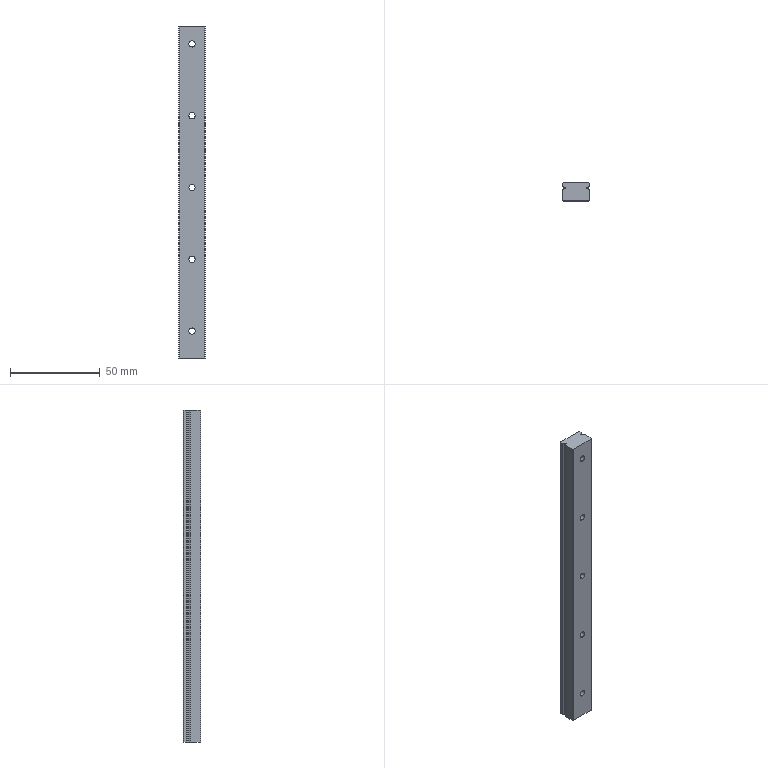Part | SolidWorks | features ICE 18, MirrorSolid 4, Extrusion 3, Fillet 3, MirrorPattern 3, RevCut 3, Chamfer 2, Dome 2, DeleteBody 1, LPattern 1, LibraryFeature 1, MoveFace 1 | 1 solid | 51 faces | box 15 x 10 x 185 mm | volume 26054 mm3 | cylinder 28 | plane 23 | commonest cylinder face diameters 3.5 x10 6 x10 0.3 x4 2.372 x4
STEP:
#1=CARTESIAN_POINT('',(0.,1.5,-83.));
#2=VERTEX_POINT('',#1);
#3=CARTESIAN_POINT('',(0.,1.5,-77.));
#4=VERTEX_POINT('',#3);
#5=CARTESIAN_POINT('',(0.,1.5,-80.));
#6=DIRECTION('',(0.,1.,0.));
#7=DIRECTION('',(0.,0.,1.));
#8=AXIS2_PLACEMENT_3D('',#5,#6,#7);
#9=CIRCLE('',#8,3.);
#10=EDGE_CURVE('',#2,#4,#9,.T.);
#11=ORIENTED_EDGE('',*,*,#10,.F.);
#12=CARTESIAN_POINT('',(0.,6.,-83.));
#13=VERTEX_POINT('',#12);
#14=CARTESIAN_POINT('',(0.,6.,-83.));
#15=DIRECTION('',(0.,1.,0.));
#16=VECTOR('',#15,1000.);
#17=LINE('',#14,#16);
#18=EDGE_CURVE('',#2,#13,#17,.T.);
#19=ORIENTED_EDGE('',*,*,#18,.T.);
#20=CARTESIAN_POINT('',(0.,6.,-77.));
#21=VERTEX_POINT('',#20);
#22=CARTESIAN_POINT('',(0.,6.,-80.));
#23=DIRECTION('',(0.,1.,0.));
#24=DIRECTION('',(0.,0.,1.));
#25=AXIS2_PLACEMENT_3D('',#22,#23,#24);
#26=CIRCLE('',#25,3.);
#27=EDGE_CURVE('',#13,#21,#26,.T.);
#28=ORIENTED_EDGE('',*,*,#27,.T.);
#29=CARTESIAN_POINT('',(0.,6.,-77.));
#30=DIRECTION('',(0.,1.,0.));
#31=VECTOR('',#30,1000.);
#32=LINE('',#29,#31);
#33=EDGE_CURVE('',#4,#21,#32,.T.);
#34=ORIENTED_EDGE('',*,*,#33,.F.);
#35=EDGE_LOOP('',(#11,#19,#28,#34));
#36=FACE_OUTER_BOUND('',#35,.T.);
#37=CARTESIAN_POINT('',(0.,6.,-80.));
#38=DIRECTION('',(0.,1.,0.));
#39=DIRECTION('',(0.,0.,1.));
#40=AXIS2_PLACEMENT_3D('',#37,#38,#39);
#41=CYLINDRICAL_SURFACE('',#40,3.);
#42=ADVANCED_FACE('',(#36),#41,.F.);
#43=CARTESIAN_POINT('',(0.,-4.,-81.75));
#44=VERTEX_POINT('',#43);
#45=CARTESIAN_POINT('',(0.,-4.,-78.25));
#46=VERTEX_POINT('',#45);
#47=CARTESIAN_POINT('',(0.,-4.,-80.));
#48=DIRECTION('',(0.,1.,0.));
#49=DIRECTION('',(0.,0.,1.));
#50=AXIS2_PLACEMENT_3D('',#47,#48,#49);
#51=CIRCLE('',#50,1.75);
#52=EDGE_CURVE('',#44,#46,#51,.T.);
#53=ORIENTED_EDGE('',*,*,#52,.F.);
#54=CARTESIAN_POINT('',(0.,1.5,-81.75));
#55=VERTEX_POINT('',#54);
#56=CARTESIAN_POINT('',(0.,6.,-81.75));
#57=DIRECTION('',(0.,1.,0.));
#58=VECTOR('',#57,1000.);
#59=LINE('',#56,#58);
#60=EDGE_CURVE('',#44,#55,#59,.T.);
#61=ORIENTED_EDGE('',*,*,#60,.T.);
#62=CARTESIAN_POINT('',(0.,1.5,-78.25));
#63=VERTEX_POINT('',#62);
#64=CARTESIAN_POINT('',(0.,1.5,-80.));
#65=DIRECTION('',(0.,1.,0.));
#66=DIRECTION('',(0.,0.,1.));
#67=AXIS2_PLACEMENT_3D('',#64,#65,#66);
#68=CIRCLE('',#67,1.75);
#69=EDGE_CURVE('',#55,#63,#68,.T.);
#70=ORIENTED_EDGE('',*,*,#69,.T.);
#71=CARTESIAN_POINT('',(0.,6.,-78.25));
#72=DIRECTION('',(0.,1.,0.));
#73=VECTOR('',#72,1000.);
#74=LINE('',#71,#73);
#75=EDGE_CURVE('',#46,#63,#74,.T.);
#76=ORIENTED_EDGE('',*,*,#75,.F.);
#77=EDGE_LOOP('',(#53,#61,#70,#76));
#78=FACE_OUTER_BOUND('',#77,.T.);
#79=CARTESIAN_POINT('',(0.,6.,-80.));
#80=DIRECTION('',(0.,1.,0.));
#81=DIRECTION('',(0.,0.,1.));
#82=AXIS2_PLACEMENT_3D('',#79,#80,#81);
#83=CYLINDRICAL_SURFACE('',#82,1.75);
#84=ADVANCED_FACE('',(#78),#83,.F.);
#85=CARTESIAN_POINT('',(0.,1.5,-43.));
#86=VERTEX_POINT('',#85);
#87=CARTESIAN_POINT('',(0.,1.5,-37.));
#88=VERTEX_POINT('',#87);
#89=CARTESIAN_POINT('',(0.,1.5,-40.));
#90=DIRECTION('',(0.,1.,0.));
#91=DIRECTION('',(0.,0.,1.));
#92=AXIS2_PLACEMENT_3D('',#89,#90,#91);
#93=CIRCLE('',#92,3.);
#94=EDGE_CURVE('',#86,#88,#93,.T.);
#95=ORIENTED_EDGE('',*,*,#94,.F.);
#96=CARTESIAN_POINT('',(0.,6.,-43.));
#97=VERTEX_POINT('',#96);
#98=CARTESIAN_POINT('',(0.,6.,-43.));
#99=DIRECTION('',(0.,1.,0.));
#100=VECTOR('',#99,1000.);
#101=LINE('',#98,#100);
#102=EDGE_CURVE('',#86,#97,#101,.T.);
#103=ORIENTED_EDGE('',*,*,#102,.T.);
#104=CARTESIAN_POINT('',(0.,6.,-37.));
#105=VERTEX_POINT('',#104);
#106=CARTESIAN_POINT('',(0.,6.,-40.));
#107=DIRECTION('',(0.,1.,0.));
#108=DIRECTION('',(0.,0.,1.));
#109=AXIS2_PLACEMENT_3D('',#106,#107,#108);
#110=CIRCLE('',#109,3.);
#111=EDGE_CURVE('',#97,#105,#110,.T.);
#112=ORIENTED_EDGE('',*,*,#111,.T.);
#113=CARTESIAN_POINT('',(0.,6.,-37.));
#114=DIRECTION('',(0.,1.,0.));
#115=VECTOR('',#114,1000.);
#116=LINE('',#113,#115);
#117=EDGE_CURVE('',#88,#105,#116,.T.);
#118=ORIENTED_EDGE('',*,*,#117,.F.);
#119=EDGE_LOOP('',(#95,#103,#112,#118));
#120=FACE_OUTER_BOUND('',#119,.T.);
#121=CARTESIAN_POINT('',(0.,6.,-40.));
#122=DIRECTION('',(0.,1.,0.));
#123=DIRECTION('',(0.,0.,1.));
#124=AXIS2_PLACEMENT_3D('',#121,#122,#123);
#125=CYLINDRICAL_SURFACE('',#124,3.);
#126=ADVANCED_FACE('',(#120),#125,.F.);
#127=CARTESIAN_POINT('',(0.,-4.,-41.75));
#128=VERTEX_POINT('',#127);
#129=CARTESIAN_POINT('',(0.,-4.,-38.25));
#130=VERTEX_POINT('',#129);
#131=CARTESIAN_POINT('',(0.,-4.,-40.));
#132=DIRECTION('',(0.,1.,0.));
#133=DIRECTION('',(0.,0.,1.));
#134=AXIS2_PLACEMENT_3D('',#131,#132,#133);
#135=CIRCLE('',#134,1.75);
#136=EDGE_CURVE('',#128,#130,#135,.T.);
#137=ORIENTED_EDGE('',*,*,#136,.F.);
#138=CARTESIAN_POINT('',(0.,1.5,-41.75));
#139=VERTEX_POINT('',#138);
#140=CARTESIAN_POINT('',(0.,6.,-41.75));
#141=DIRECTION('',(0.,1.,0.));
#142=VECTOR('',#141,1000.);
#143=LINE('',#140,#142);
#144=EDGE_CURVE('',#128,#139,#143,.T.);
#145=ORIENTED_EDGE('',*,*,#144,.T.);
#146=CARTESIAN_POINT('',(0.,1.5,-38.25));
#147=VERTEX_POINT('',#146);
#148=CARTESIAN_POINT('',(0.,1.5,-40.));
#149=DIRECTION('',(0.,1.,0.));
#150=DIRECTION('',(0.,0.,1.));
#151=AXIS2_PLACEMENT_3D('',#148,#149,#150);
#152=CIRCLE('',#151,1.75);
#153=EDGE_CURVE('',#139,#147,#152,.T.);
#154=ORIENTED_EDGE('',*,*,#153,.T.);
#155=CARTESIAN_POINT('',(0.,6.,-38.25));
#156=DIRECTION('',(0.,1.,0.));
#157=VECTOR('',#156,1000.);
#158=LINE('',#155,#157);
#159=EDGE_CURVE('',#130,#147,#158,.T.);
#160=ORIENTED_EDGE('',*,*,#159,.F.);
#161=EDGE_LOOP('',(#137,#145,#154,#160));
#162=FACE_OUTER_BOUND('',#161,.T.);
#163=CARTESIAN_POINT('',(0.,6.,-40.));
#164=DIRECTION('',(0.,1.,0.));
#165=DIRECTION('',(0.,0.,1.));
#166=AXIS2_PLACEMENT_3D('',#163,#164,#165);
#167=CYLINDRICAL_SURFACE('',#166,1.75);
#168=ADVANCED_FACE('',(#162),#167,.F.);
#169=CARTESIAN_POINT('',(0.,1.5,-3.));
#170=VERTEX_POINT('',#169);
#171=CARTESIAN_POINT('',(0.,1.5,3.));
#172=VERTEX_POINT('',#171);
#173=CARTESIAN_POINT('',(0.,1.5,0.));
#174=DIRECTION('',(0.,1.,0.));
#175=DIRECTION('',(0.,0.,1.));
#176=AXIS2_PLACEMENT_3D('',#173,#174,#175);
#177=CIRCLE('',#176,3.);
#178=EDGE_CURVE('',#170,#172,#177,.T.);
#179=ORIENTED_EDGE('',*,*,#178,.F.);
#180=CARTESIAN_POINT('',(0.,6.,-3.));
#181=VERTEX_POINT('',#180);
#182=CARTESIAN_POINT('',(0.,6.,-3.));
#183=DIRECTION('',(0.,1.,0.));
#184=VECTOR('',#183,1000.);
#185=LINE('',#182,#184);
#186=EDGE_CURVE('',#170,#181,#185,.T.);
#187=ORIENTED_EDGE('',*,*,#186,.T.);
#188=CARTESIAN_POINT('',(0.,6.,3.));
#189=VERTEX_POINT('',#188);
#190=CARTESIAN_POINT('',(0.,6.,0.));
#191=DIRECTION('',(0.,1.,0.));
#192=DIRECTION('',(0.,0.,1.));
#193=AXIS2_PLACEMENT_3D('',#190,#191,#192);
#194=CIRCLE('',#193,3.);
#195=EDGE_CURVE('',#181,#189,#194,.T.);
#196=ORIENTED_EDGE('',*,*,#195,.T.);
#197=CARTESIAN_POINT('',(0.,6.,3.));
#198=DIRECTION('',(0.,1.,0.));
#199=VECTOR('',#198,1000.);
#200=LINE('',#197,#199);
#201=EDGE_CURVE('',#172,#189,#200,.T.);
#202=ORIENTED_EDGE('',*,*,#201,.F.);
#203=EDGE_LOOP('',(#179,#187,#196,#202));
#204=FACE_OUTER_BOUND('',#203,.T.);
#205=CARTESIAN_POINT('',(0.,6.,0.));
#206=DIRECTION('',(0.,1.,0.));
#207=DIRECTION('',(0.,0.,1.));
#208=AXIS2_PLACEMENT_3D('',#205,#206,#207);
#209=CYLINDRICAL_SURFACE('',#208,3.);
#210=ADVANCED_FACE('',(#204),#209,.F.);
#211=CARTESIAN_POINT('',(0.,-4.,-1.75));
#212=VERTEX_POINT('',#211);
#213=CARTESIAN_POINT('',(0.,-4.,1.75));
#214=VERTEX_POINT('',#213);
#215=CARTESIAN_POINT('',(0.,-4.,0.));
#216=DIRECTION('',(0.,1.,0.));
#217=DIRECTION('',(0.,0.,1.));
#218=AXIS2_PLACEMENT_3D('',#215,#216,#217);
#219=CIRCLE('',#218,1.75);
#220=EDGE_CURVE('',#212,#214,#219,.T.);
#221=ORIENTED_EDGE('',*,*,#220,.F.);
#222=CARTESIAN_POINT('',(0.,1.5,-1.75));
#223=VERTEX_POINT('',#222);
#224=CARTESIAN_POINT('',(0.,6.,-1.75));
#225=DIRECTION('',(0.,1.,0.));
#226=VECTOR('',#225,1000.);
#227=LINE('',#224,#226);
#228=EDGE_CURVE('',#212,#223,#227,.T.);
#229=ORIENTED_EDGE('',*,*,#228,.T.);
#230=CARTESIAN_POINT('',(0.,1.5,1.75));
#231=VERTEX_POINT('',#230);
#232=CARTESIAN_POINT('',(0.,1.5,0.));
#233=DIRECTION('',(0.,1.,0.));
#234=DIRECTION('',(0.,0.,1.));
#235=AXIS2_PLACEMENT_3D('',#232,#233,#234);
#236=CIRCLE('',#235,1.75);
#237=EDGE_CURVE('',#223,#231,#236,.T.);
#238=ORIENTED_EDGE('',*,*,#237,.T.);
#239=CARTESIAN_POINT('',(0.,6.,1.75));
#240=DIRECTION('',(0.,1.,0.));
#241=VECTOR('',#240,1000.);
#242=LINE('',#239,#241);
#243=EDGE_CURVE('',#214,#231,#242,.T.);
#244=ORIENTED_EDGE('',*,*,#243,.F.);
#245=EDGE_LOOP('',(#221,#229,#238,#244));
#246=FACE_OUTER_BOUND('',#245,.T.);
#247=CARTESIAN_POINT('',(0.,6.,0.));
#248=DIRECTION('',(0.,1.,0.));
#249=DIRECTION('',(0.,0.,1.));
#250=AXIS2_PLACEMENT_3D('',#247,#248,#249);
#251=CYLINDRICAL_SURFACE('',#250,1.75);
#252=ADVANCED_FACE('',(#246),#251,.F.);
#253=CARTESIAN_POINT('',(0.,1.5,37.));
#254=VERTEX_POINT('',#253);
#255=CARTESIAN_POINT('',(0.,1.5,43.));
#256=VERTEX_POINT('',#255);
#257=CARTESIAN_POINT('',(0.,1.5,40.));
#258=DIRECTION('',(0.,1.,0.));
#259=DIRECTION('',(0.,0.,1.));
#260=AXIS2_PLACEMENT_3D('',#257,#258,#259);
#261=CIRCLE('',#260,3.);
#262=EDGE_CURVE('',#254,#256,#261,.T.);
#263=ORIENTED_EDGE('',*,*,#262,.F.);
#264=CARTESIAN_POINT('',(0.,6.,37.));
#265=VERTEX_POINT('',#264);
#266=CARTESIAN_POINT('',(0.,6.,37.));
#267=DIRECTION('',(0.,1.,0.));
#268=VECTOR('',#267,1000.);
#269=LINE('',#266,#268);
#270=EDGE_CURVE('',#254,#265,#269,.T.);
#271=ORIENTED_EDGE('',*,*,#270,.T.);
#272=CARTESIAN_POINT('',(0.,6.,43.));
#273=VERTEX_POINT('',#272);
#274=CARTESIAN_POINT('',(0.,6.,40.));
#275=DIRECTION('',(0.,1.,0.));
#276=DIRECTION('',(0.,0.,1.));
#277=AXIS2_PLACEMENT_3D('',#274,#275,#276);
#278=CIRCLE('',#277,3.);
#279=EDGE_CURVE('',#265,#273,#278,.T.);
#280=ORIENTED_EDGE('',*,*,#279,.T.);
#281=CARTESIAN_POINT('',(0.,6.,43.));
#282=DIRECTION('',(0.,1.,0.));
#283=VECTOR('',#282,1000.);
#284=LINE('',#281,#283);
#285=EDGE_CURVE('',#256,#273,#284,.T.);
#286=ORIENTED_EDGE('',*,*,#285,.F.);
#287=EDGE_LOOP('',(#263,#271,#280,#286));
#288=FACE_OUTER_BOUND('',#287,.T.);
#289=CARTESIAN_POINT('',(0.,6.,40.));
#290=DIRECTION('',(0.,1.,0.));
#291=DIRECTION('',(0.,0.,1.));
#292=AXIS2_PLACEMENT_3D('',#289,#290,#291);
#293=CYLINDRICAL_SURFACE('',#292,3.);
#294=ADVANCED_FACE('',(#288),#293,.F.);
#295=CARTESIAN_POINT('',(0.,-4.,38.25));
#296=VERTEX_POINT('',#295);
#297=CARTESIAN_POINT('',(0.,-4.,41.75));
#298=VERTEX_POINT('',#297);
#299=CARTESIAN_POINT('',(0.,-4.,40.));
#300=DIRECTION('',(0.,1.,0.));
#301=DIRECTION('',(0.,0.,1.));
#302=AXIS2_PLACEMENT_3D('',#299,#300,#301);
#303=CIRCLE('',#302,1.75);
#304=EDGE_CURVE('',#296,#298,#303,.T.);
#305=ORIENTED_EDGE('',*,*,#304,.F.);
#306=CARTESIAN_POINT('',(0.,1.5,38.25));
#307=VERTEX_POINT('',#306);
#308=CARTESIAN_POINT('',(0.,6.,38.25));
#309=DIRECTION('',(0.,1.,0.));
#310=VECTOR('',#309,1000.);
#311=LINE('',#308,#310);
#312=EDGE_CURVE('',#296,#307,#311,.T.);
#313=ORIENTED_EDGE('',*,*,#312,.T.);
#314=CARTESIAN_POINT('',(0.,1.5,41.75));
#315=VERTEX_POINT('',#314);
#316=CARTESIAN_POINT('',(0.,1.5,40.));
#317=DIRECTION('',(0.,1.,0.));
#318=DIRECTION('',(0.,0.,1.));
#319=AXIS2_PLACEMENT_3D('',#316,#317,#318);
#320=CIRCLE('',#319,1.75);
#321=EDGE_CURVE('',#307,#315,#320,.T.);
#322=ORIENTED_EDGE('',*,*,#321,.T.);
#323=CARTESIAN_POINT('',(0.,6.,41.75));
#324=DIRECTION('',(0.,1.,0.));
#325=VECTOR('',#324,1000.);
#326=LINE('',#323,#325);
#327=EDGE_CURVE('',#298,#315,#326,.T.);
#328=ORIENTED_EDGE('',*,*,#327,.F.);
#329=EDGE_LOOP('',(#305,#313,#322,#328));
#330=FACE_OUTER_BOUND('',#329,.T.);
#331=CARTESIAN_POINT('',(0.,6.,40.));
#332=DIRECTION('',(0.,1.,0.));
#333=DIRECTION('',(0.,0.,1.));
#334=AXIS2_PLACEMENT_3D('',#331,#332,#333);
#335=CYLINDRICAL_SURFACE('',#334,1.75);
#336=ADVANCED_FACE('',(#330),#335,.F.);
#337=CARTESIAN_POINT('',(0.,1.5,77.));
#338=VERTEX_POINT('',#337);
#339=CARTESIAN_POINT('',(0.,1.5,83.));
#340=VERTEX_POINT('',#339);
#341=CARTESIAN_POINT('',(0.,1.5,80.));
#342=DIRECTION('',(0.,1.,0.));
#343=DIRECTION('',(0.,0.,1.));
#344=AXIS2_PLACEMENT_3D('',#341,#342,#343);
#345=CIRCLE('',#344,3.);
#346=EDGE_CURVE('',#338,#340,#345,.T.);
#347=ORIENTED_EDGE('',*,*,#346,.F.);
#348=CARTESIAN_POINT('',(0.,6.,77.));
#349=VERTEX_POINT('',#348);
#350=CARTESIAN_POINT('',(0.,6.,77.));
#351=DIRECTION('',(0.,1.,0.));
#352=VECTOR('',#351,1000.);
#353=LINE('',#350,#352);
#354=EDGE_CURVE('',#338,#349,#353,.T.);
#355=ORIENTED_EDGE('',*,*,#354,.T.);
#356=CARTESIAN_POINT('',(0.,6.,83.));
#357=VERTEX_POINT('',#356);
#358=CARTESIAN_POINT('',(0.,6.,80.));
#359=DIRECTION('',(0.,1.,0.));
#360=DIRECTION('',(0.,0.,1.));
#361=AXIS2_PLACEMENT_3D('',#358,#359,#360);
#362=CIRCLE('',#361,3.);
#363=EDGE_CURVE('',#349,#357,#362,.T.);
#364=ORIENTED_EDGE('',*,*,#363,.T.);
#365=CARTESIAN_POINT('',(0.,6.,83.));
#366=DIRECTION('',(0.,1.,0.));
#367=VECTOR('',#366,1000.);
#368=LINE('',#365,#367);
#369=EDGE_CURVE('',#340,#357,#368,.T.);
#370=ORIENTED_EDGE('',*,*,#369,.F.);
#371=EDGE_LOOP('',(#347,#355,#364,#370));
#372=FACE_OUTER_BOUND('',#371,.T.);
#373=CARTESIAN_POINT('',(0.,6.,80.));
#374=DIRECTION('',(0.,1.,0.));
#375=DIRECTION('',(0.,0.,1.));
#376=AXIS2_PLACEMENT_3D('',#373,#374,#375);
#377=CYLINDRICAL_SURFACE('',#376,3.);
#378=ADVANCED_FACE('',(#372),#377,.F.);
#379=CARTESIAN_POINT('',(0.,-4.,78.25));
#380=VERTEX_POINT('',#379);
#381=CARTESIAN_POINT('',(0.,-4.,81.75));
#382=VERTEX_POINT('',#381);
#383=CARTESIAN_POINT('',(0.,-4.,80.));
#384=DIRECTION('',(0.,1.,0.));
#385=DIRECTION('',(0.,0.,1.));
#386=AXIS2_PLACEMENT_3D('',#383,#384,#385);
#387=CIRCLE('',#386,1.75);
#388=EDGE_CURVE('',#380,#382,#387,.T.);
#389=ORIENTED_EDGE('',*,*,#388,.F.);
#390=CARTESIAN_POINT('',(0.,1.5,78.25));
#391=VERTEX_POINT('',#390);
#392=CARTESIAN_POINT('',(0.,6.,78.25));
#393=DIRECTION('',(0.,1.,0.));
#394=VECTOR('',#393,1000.);
#395=LINE('',#392,#394);
#396=EDGE_CURVE('',#380,#391,#395,.T.);
#397=ORIENTED_EDGE('',*,*,#396,.T.);
#398=CARTESIAN_POINT('',(0.,1.5,81.75));
#399=VERTEX_POINT('',#398);
#400=CARTESIAN_POINT('',(0.,1.5,80.));
#401=DIRECTION('',(0.,1.,0.));
#402=DIRECTION('',(0.,0.,1.));
#403=AXIS2_PLACEMENT_3D('',#400,#401,#402);
#404=CIRCLE('',#403,1.75);
#405=EDGE_CURVE('',#391,#399,#404,.T.);
#406=ORIENTED_EDGE('',*,*,#405,.T.);
#407=CARTESIAN_POINT('',(0.,6.,81.75));
#408=DIRECTION('',(0.,1.,0.));
#409=VECTOR('',#408,1000.);
#410=LINE('',#407,#409);
#411=EDGE_CURVE('',#382,#399,#410,.T.);
#412=ORIENTED_EDGE('',*,*,#411,.F.);
#413=EDGE_LOOP('',(#389,#397,#406,#412));
#414=FACE_OUTER_BOUND('',#413,.T.);
#415=CARTESIAN_POINT('',(0.,6.,80.));
#416=DIRECTION('',(0.,1.,0.));
#417=DIRECTION('',(0.,0.,1.));
#418=AXIS2_PLACEMENT_3D('',#415,#416,#417);
#419=CYLINDRICAL_SURFACE('',#418,1.75);
#420=ADVANCED_FACE('',(#414),#419,.F.);
#421=CARTESIAN_POINT('',(7.5,5.55,90.));
#422=VERTEX_POINT('',#421);
#423=CARTESIAN_POINT('',(7.5,5.55,-95.));
#424=VERTEX_POINT('',#423);
#425=CARTESIAN_POINT('',(7.5,5.55,90.));
#426=DIRECTION('',(0.,0.,-1.));
#427=VECTOR('',#426,1000.);
#428=LINE('',#425,#427);
#429=EDGE_CURVE('',#422,#424,#428,.T.);
#430=ORIENTED_EDGE('',*,*,#429,.T.);
#431=CARTESIAN_POINT('',(7.05,6.,-95.));
#432=VERTEX_POINT('',#431);
#433=CARTESIAN_POINT('',(7.5,5.55,-95.));
#434=DIRECTION('',(-0.7071,0.7071,0.));
#435=VECTOR('',#434,1000.);
#436=LINE('',#433,#435);
#437=EDGE_CURVE('',#424,#432,#436,.T.);
#438=ORIENTED_EDGE('',*,*,#437,.T.);
#439=CARTESIAN_POINT('',(7.05,6.,90.));
#440=VERTEX_POINT('',#439);
#441=CARTESIAN_POINT('',(7.05,6.,90.));
#442=DIRECTION('',(0.,0.,-1.));
#443=VECTOR('',#442,1000.);
#444=LINE('',#441,#443);
#445=EDGE_CURVE('',#440,#432,#444,.T.);
#446=ORIENTED_EDGE('',*,*,#445,.F.);
#447=CARTESIAN_POINT('',(7.5,5.55,90.));
#448=DIRECTION('',(-0.7071,0.7071,0.));
#449=VECTOR('',#448,1000.);
#450=LINE('',#447,#449);
#451=EDGE_CURVE('',#422,#440,#450,.T.);
#452=ORIENTED_EDGE('',*,*,#451,.F.);
#453=EDGE_LOOP('',(#430,#438,#446,#452));
#454=FACE_OUTER_BOUND('',#453,.T.);
#455=CARTESIAN_POINT('',(7.5,5.55,90.));
#456=DIRECTION('',(-0.7071,-0.7071,0.));
#457=DIRECTION('',(0.7071,-0.7071,0.));
#458=AXIS2_PLACEMENT_3D('',#455,#456,#457);
#459=PLANE('',#458);
#460=ADVANCED_FACE('',(#454),#459,.F.);
#461=CARTESIAN_POINT('',(0.,6.,-80.));
#462=DIRECTION('',(0.,1.,0.));
#463=DIRECTION('',(0.,0.,1.));
#464=AXIS2_PLACEMENT_3D('',#461,#462,#463);
#465=CIRCLE('',#464,3.);
#466=EDGE_CURVE('',#21,#13,#465,.T.);
#467=ORIENTED_EDGE('',*,*,#466,.F.);
#468=ORIENTED_EDGE('',*,*,#27,.F.);
#469=EDGE_LOOP('',(#467,#468));
#470=FACE_BOUND('',#469,.T.);
#471=CARTESIAN_POINT('',(0.,6.,-40.));
#472=DIRECTION('',(0.,1.,0.));
#473=DIRECTION('',(0.,0.,1.));
#474=AXIS2_PLACEMENT_3D('',#471,#472,#473);
#475=CIRCLE('',#474,3.);
#476=EDGE_CURVE('',#105,#97,#475,.T.);
#477=ORIENTED_EDGE('',*,*,#476,.F.);
#478=ORIENTED_EDGE('',*,*,#111,.F.);
#479=EDGE_LOOP('',(#477,#478));
#480=FACE_BOUND('',#479,.T.);
#481=CARTESIAN_POINT('',(0.,6.,0.));
#482=DIRECTION('',(0.,1.,0.));
#483=DIRECTION('',(0.,0.,1.));
#484=AXIS2_PLACEMENT_3D('',#481,#482,#483);
#485=CIRCLE('',#484,3.);
#486=EDGE_CURVE('',#189,#181,#485,.T.);
#487=ORIENTED_EDGE('',*,*,#486,.F.);
#488=ORIENTED_EDGE('',*,*,#195,.F.);
#489=EDGE_LOOP('',(#487,#488));
#490=FACE_BOUND('',#489,.T.);
#491=CARTESIAN_POINT('',(0.,6.,40.));
#492=DIRECTION('',(0.,1.,0.));
#493=DIRECTION('',(0.,0.,1.));
#494=AXIS2_PLACEMENT_3D('',#491,#492,#493);
#495=CIRCLE('',#494,3.);
#496=EDGE_CURVE('',#273,#265,#495,.T.);
#497=ORIENTED_EDGE('',*,*,#496,.F.);
#498=ORIENTED_EDGE('',*,*,#279,.F.);
#499=EDGE_LOOP('',(#497,#498));
#500=FACE_BOUND('',#499,.T.);
#501=CARTESIAN_POINT('',(0.,6.,80.));
#502=DIRECTION('',(0.,1.,0.));
#503=DIRECTION('',(0.,0.,1.));
#504=AXIS2_PLACEMENT_3D('',#501,#502,#503);
#505=CIRCLE('',#504,3.);
#506=EDGE_CURVE('',#357,#349,#505,.T.);
#507=ORIENTED_EDGE('',*,*,#506,.F.);
#508=ORIENTED_EDGE('',*,*,#363,.F.);
#509=EDGE_LOOP('',(#507,#508));
#510=FACE_BOUND('',#509,.T.);
#511=ORIENTED_EDGE('',*,*,#445,.T.);
#512=CARTESIAN_POINT('',(-7.05,6.,-95.));
#513=VERTEX_POINT('',#512);
#514=CARTESIAN_POINT('',(7.05,6.,-95.));
#515=DIRECTION('',(-1.,0.,0.));
#516=VECTOR('',#515,1000.);
#517=LINE('',#514,#516);
#518=EDGE_CURVE('',#432,#513,#517,.T.);
#519=ORIENTED_EDGE('',*,*,#518,.T.);
#520=CARTESIAN_POINT('',(-7.05,6.,90.));
#521=VERTEX_POINT('',#520);
#522=CARTESIAN_POINT('',(-7.05,6.,90.));
#523=DIRECTION('',(0.,0.,-1.));
#524=VECTOR('',#523,1000.);
#525=LINE('',#522,#524);
#526=EDGE_CURVE('',#521,#513,#525,.T.);
#527=ORIENTED_EDGE('',*,*,#526,.F.);
#528=CARTESIAN_POINT('',(7.05,6.,90.));
#529=DIRECTION('',(-1.,0.,0.));
#530=VECTOR('',#529,1000.);
#531=LINE('',#528,#530);
#532=EDGE_CURVE('',#440,#521,#531,.T.);
#533=ORIENTED_EDGE('',*,*,#532,.F.);
#534=EDGE_LOOP('',(#511,#519,#527,#533));
#535=FACE_OUTER_BOUND('',#534,.T.);
#536=CARTESIAN_POINT('',(7.05,6.,90.));
#537=DIRECTION('',(0.,-1.,0.));
#538=DIRECTION('',(0.,0.,-1.));
#539=AXIS2_PLACEMENT_3D('',#536,#537,#538);
#540=PLANE('',#539);
#541=ADVANCED_FACE('',(#470,#480,#490,#500,#510,#535),#540,.F.);
#542=ORIENTED_EDGE('',*,*,#526,.T.);
#543=CARTESIAN_POINT('',(-7.5,5.55,-95.));
#544=VERTEX_POINT('',#543);
#545=CARTESIAN_POINT('',(-7.5,5.55,-95.));
#546=DIRECTION('',(-0.7071,-0.7071,0.));
#547=VECTOR('',#546,1000.);
#548=LINE('',#545,#547);
#549=EDGE_CURVE('',#513,#544,#548,.T.);
#550=ORIENTED_EDGE('',*,*,#549,.T.);
#551=CARTESIAN_POINT('',(-7.5,5.55,90.));
#552=VERTEX_POINT('',#551);
#553=CARTESIAN_POINT('',(-7.5,5.55,90.));
#554=DIRECTION('',(0.,0.,-1.));
#555=VECTOR('',#554,1000.);
#556=LINE('',#553,#555);
#557=EDGE_CURVE('',#552,#544,#556,.T.);
#558=ORIENTED_EDGE('',*,*,#557,.F.);
#559=CARTESIAN_POINT('',(-7.5,5.55,90.));
#560=DIRECTION('',(-0.7071,-0.7071,0.));
#561=VECTOR('',#560,1000.);
#562=LINE('',#559,#561);
#563=EDGE_CURVE('',#521,#552,#562,.T.);
#564=ORIENTED_EDGE('',*,*,#563,.F.);
#565=EDGE_LOOP('',(#542,#550,#558,#564));
#566=FACE_OUTER_BOUND('',#565,.T.);
#567=CARTESIAN_POINT('',(-7.5,5.55,90.));
#568=DIRECTION('',(0.7071,-0.7071,0.));
#569=DIRECTION('',(0.7071,0.7071,0.));
#570=AXIS2_PLACEMENT_3D('',#567,#568,#569);
#571=PLANE('',#570);
#572=ADVANCED_FACE('',(#566),#571,.F.);
#573=ORIENTED_EDGE('',*,*,#557,.T.);
#574=CARTESIAN_POINT('',(-7.5,4.125,-95.));
#575=VERTEX_POINT('',#574);
#576=CARTESIAN_POINT('',(-7.5,4.125,-95.));
#577=DIRECTION('',(0.,-1.,0.));
#578=VECTOR('',#577,1000.);
#579=LINE('',#576,#578);
#580=EDGE_CURVE('',#544,#575,#579,.T.);
#581=ORIENTED_EDGE('',*,*,#580,.T.);
#582=CARTESIAN_POINT('',(-7.5,4.125,90.));
#583=VERTEX_POINT('',#582);
#584=CARTESIAN_POINT('',(-7.5,4.125,90.));
#585=DIRECTION('',(0.,0.,-1.));
#586=VECTOR('',#585,1000.);
#587=LINE('',#584,#586);
#588=EDGE_CURVE('',#583,#575,#587,.T.);
#589=ORIENTED_EDGE('',*,*,#588,.F.);
#590=CARTESIAN_POINT('',(-7.5,4.125,90.));
#591=DIRECTION('',(0.,-1.,0.));
#592=VECTOR('',#591,1000.);
#593=LINE('',#590,#592);
#594=EDGE_CURVE('',#552,#583,#593,.T.);
#595=ORIENTED_EDGE('',*,*,#594,.F.);
#596=EDGE_LOOP('',(#573,#581,#589,#595));
#597=FACE_OUTER_BOUND('',#596,.T.);
#598=CARTESIAN_POINT('',(-7.5,4.125,90.));
#599=DIRECTION('',(1.,0.,0.));
#600=DIRECTION('',(0.,0.,-1.));
#601=AXIS2_PLACEMENT_3D('',#598,#599,#600);
#602=PLANE('',#601);
#603=ADVANCED_FACE('',(#597),#602,.F.);
#604=ORIENTED_EDGE('',*,*,#588,.T.);
#605=CARTESIAN_POINT('',(-6.778,3.45,-95.));
#606=VERTEX_POINT('',#605);
#607=CARTESIAN_POINT('',(-7.875,3.,-95.));
#608=DIRECTION('',(0.,0.,-1.));
#609=DIRECTION('',(1.,0.,0.));
#610=AXIS2_PLACEMENT_3D('',#607,#608,#609);
#611=CIRCLE('',#610,1.186);
#612=EDGE_CURVE('',#575,#606,#611,.T.);
#613=ORIENTED_EDGE('',*,*,#612,.T.);
#614=CARTESIAN_POINT('',(-6.778,3.45,90.));
#615=VERTEX_POINT('',#614);
#616=CARTESIAN_POINT('',(-6.778,3.45,90.));
#617=DIRECTION('',(0.,0.,-1.));
#618=VECTOR('',#617,1000.);
#619=LINE('',#616,#618);
#620=EDGE_CURVE('',#615,#606,#619,.T.);
#621=ORIENTED_EDGE('',*,*,#620,.F.);
#622=CARTESIAN_POINT('',(-7.875,3.,90.));
#623=DIRECTION('',(0.,0.,-1.));
#624=DIRECTION('',(1.,0.,0.));
#625=AXIS2_PLACEMENT_3D('',#622,#623,#624);
#626=CIRCLE('',#625,1.186);
#627=EDGE_CURVE('',#583,#615,#626,.T.);
#628=ORIENTED_EDGE('',*,*,#627,.F.);
#629=EDGE_LOOP('',(#604,#613,#621,#628));
#630=FACE_OUTER_BOUND('',#629,.T.);
#631=CARTESIAN_POINT('',(-7.875,3.,90.));
#632=DIRECTION('',(0.,0.,-1.));
#633=DIRECTION('',(-1.,0.,0.));
#634=AXIS2_PLACEMENT_3D('',#631,#632,#633);
#635=CYLINDRICAL_SURFACE('',#634,1.186);
#636=ADVANCED_FACE('',(#630),#635,.F.);
#637=ORIENTED_EDGE('',*,*,#620,.T.);
#638=CARTESIAN_POINT('',(-6.178,3.45,-95.));
#639=VERTEX_POINT('',#638);
#640=CARTESIAN_POINT('',(-6.778,3.45,-95.));
#641=DIRECTION('',(1.,0.,0.));
#642=VECTOR('',#641,1000.);
#643=LINE('',#640,#642);
#644=EDGE_CURVE('',#606,#639,#643,.T.);
#645=ORIENTED_EDGE('',*,*,#644,.T.);
#646=CARTESIAN_POINT('',(-6.178,3.45,90.));
#647=VERTEX_POINT('',#646);
#648=CARTESIAN_POINT('',(-6.178,3.45,90.));
#649=DIRECTION('',(0.,0.,-1.));
#650=VECTOR('',#649,1000.);
#651=LINE('',#648,#650);
#652=EDGE_CURVE('',#647,#639,#651,.T.);
#653=ORIENTED_EDGE('',*,*,#652,.F.);
#654=CARTESIAN_POINT('',(-6.778,3.45,90.));
#655=DIRECTION('',(1.,0.,0.));
#656=VECTOR('',#655,1000.);
#657=LINE('',#654,#656);
#658=EDGE_CURVE('',#615,#647,#657,.T.);
#659=ORIENTED_EDGE('',*,*,#658,.F.);
#660=EDGE_LOOP('',(#637,#645,#653,#659));
#661=FACE_OUTER_BOUND('',#660,.T.);
#662=CARTESIAN_POINT('',(-6.778,3.45,90.));
#663=DIRECTION('',(0.,1.,0.));
#664=DIRECTION('',(-1.,0.,0.));
#665=AXIS2_PLACEMENT_3D('',#662,#663,#664);
#666=PLANE('',#665);
#667=ADVANCED_FACE('',(#661),#666,.F.);
#668=ORIENTED_EDGE('',*,*,#652,.T.);
#669=CARTESIAN_POINT('',(-6.028,3.3,-95.));
#670=VERTEX_POINT('',#669);
#671=CARTESIAN_POINT('',(-6.178,3.3,-95.));
#672=DIRECTION('',(0.,0.,-1.));
#673=DIRECTION('',(1.,0.,0.));
#674=AXIS2_PLACEMENT_3D('',#671,#672,#673);
#675=CIRCLE('',#674,0.15);
#676=EDGE_CURVE('',#639,#670,#675,.T.);
#677=ORIENTED_EDGE('',*,*,#676,.T.);
#678=CARTESIAN_POINT('',(-6.028,3.3,90.));
#679=VERTEX_POINT('',#678);
#680=CARTESIAN_POINT('',(-6.028,3.3,90.));
#681=DIRECTION('',(0.,0.,-1.));
#682=VECTOR('',#681,1000.);
#683=LINE('',#680,#682);
#684=EDGE_CURVE('',#679,#670,#683,.T.);
#685=ORIENTED_EDGE('',*,*,#684,.F.);
#686=CARTESIAN_POINT('',(-6.178,3.3,90.));
#687=DIRECTION('',(0.,0.,-1.));
#688=DIRECTION('',(1.,0.,0.));
#689=AXIS2_PLACEMENT_3D('',#686,#687,#688);
#690=CIRCLE('',#689,0.15);
#691=EDGE_CURVE('',#647,#679,#690,.T.);
#692=ORIENTED_EDGE('',*,*,#691,.F.);
#693=EDGE_LOOP('',(#668,#677,#685,#692));
#694=FACE_OUTER_BOUND('',#693,.T.);
#695=CARTESIAN_POINT('',(-6.178,3.3,90.));
#696=DIRECTION('',(0.,0.,-1.));
#697=DIRECTION('',(-1.,0.,0.));
#698=AXIS2_PLACEMENT_3D('',#695,#696,#697);
#699=CYLINDRICAL_SURFACE('',#698,0.15);
#700=ADVANCED_FACE('',(#694),#699,.F.);
#701=ORIENTED_EDGE('',*,*,#684,.T.);
#702=CARTESIAN_POINT('',(-6.028,2.7,-95.));
#703=VERTEX_POINT('',#702);
#704=CARTESIAN_POINT('',(-6.028,3.3,-95.));
#705=DIRECTION('',(0.,-1.,0.));
#706=VECTOR('',#705,1000.);
#707=LINE('',#704,#706);
#708=EDGE_CURVE('',#670,#703,#707,.T.);
#709=ORIENTED_EDGE('',*,*,#708,.T.);
#710=CARTESIAN_POINT('',(-6.028,2.7,90.));
#711=VERTEX_POINT('',#710);
#712=CARTESIAN_POINT('',(-6.028,2.7,90.));
#713=DIRECTION('',(0.,0.,-1.));
#714=VECTOR('',#713,1000.);
#715=LINE('',#712,#714);
#716=EDGE_CURVE('',#711,#703,#715,.T.);
#717=ORIENTED_EDGE('',*,*,#716,.F.);
#718=CARTESIAN_POINT('',(-6.028,3.3,90.));
#719=DIRECTION('',(0.,-1.,0.));
#720=VECTOR('',#719,1000.);
#721=LINE('',#718,#720);
#722=EDGE_CURVE('',#679,#711,#721,.T.);
#723=ORIENTED_EDGE('',*,*,#722,.F.);
#724=EDGE_LOOP('',(#701,#709,#717,#723));
#725=FACE_OUTER_BOUND('',#724,.T.);
#726=CARTESIAN_POINT('',(-6.028,3.3,90.));
#727=DIRECTION('',(1.,0.,0.));
#728=DIRECTION('',(0.,1.,0.));
#729=AXIS2_PLACEMENT_3D('',#726,#727,#728);
#730=PLANE('',#729);
#731=ADVANCED_FACE('',(#725),#730,.F.);
#732=ORIENTED_EDGE('',*,*,#716,.T.);
#733=CARTESIAN_POINT('',(-6.178,2.55,-95.));
#734=VERTEX_POINT('',#733);
#735=CARTESIAN_POINT('',(-6.178,2.7,-95.));
#736=DIRECTION('',(0.,0.,-1.));
#737=DIRECTION('',(1.,0.,0.));
#738=AXIS2_PLACEMENT_3D('',#735,#736,#737);
#739=CIRCLE('',#738,0.15);
#740=EDGE_CURVE('',#703,#734,#739,.T.);
#741=ORIENTED_EDGE('',*,*,#740,.T.);
#742=CARTESIAN_POINT('',(-6.178,2.55,90.));
#743=VERTEX_POINT('',#742);
#744=CARTESIAN_POINT('',(-6.178,2.55,90.));
#745=DIRECTION('',(0.,0.,-1.));
#746=VECTOR('',#745,1000.);
#747=LINE('',#744,#746);
#748=EDGE_CURVE('',#743,#734,#747,.T.);
#749=ORIENTED_EDGE('',*,*,#748,.F.);
#750=CARTESIAN_POINT('',(-6.178,2.7,90.));
#751=DIRECTION('',(0.,0.,-1.));
#752=DIRECTION('',(1.,0.,0.));
#753=AXIS2_PLACEMENT_3D('',#750,#751,#752);
#754=CIRCLE('',#753,0.15);
#755=EDGE_CURVE('',#711,#743,#754,.T.);
#756=ORIENTED_EDGE('',*,*,#755,.F.);
#757=EDGE_LOOP('',(#732,#741,#749,#756));
#758=FACE_OUTER_BOUND('',#757,.T.);
#759=CARTESIAN_POINT('',(-6.178,2.7,90.));
#760=DIRECTION('',(0.,0.,-1.));
#761=DIRECTION('',(-1.,0.,0.));
#762=AXIS2_PLACEMENT_3D('',#759,#760,#761);
#763=CYLINDRICAL_SURFACE('',#762,0.15);
#764=ADVANCED_FACE('',(#758),#763,.F.);
#765=ORIENTED_EDGE('',*,*,#748,.T.);
#766=CARTESIAN_POINT('',(-6.778,2.55,-95.));
#767=VERTEX_POINT('',#766);
#768=CARTESIAN_POINT('',(-6.778,2.55,-95.));
#769=DIRECTION('',(-1.,0.,0.));
#770=VECTOR('',#769,1000.);
#771=LINE('',#768,#770);
#772=EDGE_CURVE('',#734,#767,#771,.T.);
#773=ORIENTED_EDGE('',*,*,#772,.T.);
#774=CARTESIAN_POINT('',(-6.778,2.55,90.));
#775=VERTEX_POINT('',#774);
#776=CARTESIAN_POINT('',(-6.778,2.55,90.));
#777=DIRECTION('',(0.,0.,-1.));
#778=VECTOR('',#777,1000.);
#779=LINE('',#776,#778);
#780=EDGE_CURVE('',#775,#767,#779,.T.);
#781=ORIENTED_EDGE('',*,*,#780,.F.);
#782=CARTESIAN_POINT('',(-6.778,2.55,90.));
#783=DIRECTION('',(-1.,0.,0.));
#784=VECTOR('',#783,1000.);
#785=LINE('',#782,#784);
#786=EDGE_CURVE('',#743,#775,#785,.T.);
#787=ORIENTED_EDGE('',*,*,#786,.F.);
#788=EDGE_LOOP('',(#765,#773,#781,#787));
#789=FACE_OUTER_BOUND('',#788,.T.);
#790=CARTESIAN_POINT('',(-6.778,2.55,90.));
#791=DIRECTION('',(0.,-1.,0.));
#792=DIRECTION('',(1.,0.,0.));
#793=AXIS2_PLACEMENT_3D('',#790,#791,#792);
#794=PLANE('',#793);
#795=ADVANCED_FACE('',(#789),#794,.F.);
#796=ORIENTED_EDGE('',*,*,#780,.T.);
#797=CARTESIAN_POINT('',(-7.5,1.875,-95.));
#798=VERTEX_POINT('',#797);
#799=CARTESIAN_POINT('',(-7.875,3.,-95.));
#800=DIRECTION('',(0.,0.,-1.));
#801=DIRECTION('',(1.,0.,0.));
#802=AXIS2_PLACEMENT_3D('',#799,#800,#801);
#803=CIRCLE('',#802,1.186);
#804=EDGE_CURVE('',#767,#798,#803,.T.);
#805=ORIENTED_EDGE('',*,*,#804,.T.);
#806=CARTESIAN_POINT('',(-7.5,1.875,90.));
#807=VERTEX_POINT('',#806);
#808=CARTESIAN_POINT('',(-7.5,1.875,90.));
#809=DIRECTION('',(0.,0.,-1.));
#810=VECTOR('',#809,1000.);
#811=LINE('',#808,#810);
#812=EDGE_CURVE('',#807,#798,#811,.T.);
#813=ORIENTED_EDGE('',*,*,#812,.F.);
#814=CARTESIAN_POINT('',(-7.875,3.,90.));
#815=DIRECTION('',(0.,0.,-1.));
#816=DIRECTION('',(1.,0.,0.));
#817=AXIS2_PLACEMENT_3D('',#814,#815,#816);
#818=CIRCLE('',#817,1.186);
#819=EDGE_CURVE('',#775,#807,#818,.T.);
#820=ORIENTED_EDGE('',*,*,#819,.F.);
#821=EDGE_LOOP('',(#796,#805,#813,#820));
#822=FACE_OUTER_BOUND('',#821,.T.);
#823=CARTESIAN_POINT('',(-7.875,3.,90.));
#824=DIRECTION('',(0.,0.,-1.));
#825=DIRECTION('',(-1.,0.,0.));
#826=AXIS2_PLACEMENT_3D('',#823,#824,#825);
#827=CYLINDRICAL_SURFACE('',#826,1.186);
#828=ADVANCED_FACE('',(#822),#827,.F.);
#829=ORIENTED_EDGE('',*,*,#812,.T.);
#830=CARTESIAN_POINT('',(-7.5,-3.55,-95.));
#831=VERTEX_POINT('',#830);
#832=CARTESIAN_POINT('',(-7.5,-3.55,-95.));
#833=DIRECTION('',(0.,-1.,0.));
#834=VECTOR('',#833,1000.);
#835=LINE('',#832,#834);
#836=EDGE_CURVE('',#798,#831,#835,.T.);
#837=ORIENTED_EDGE('',*,*,#836,.T.);
#838=CARTESIAN_POINT('',(-7.5,-3.55,90.));
#839=VERTEX_POINT('',#838);
#840=CARTESIAN_POINT('',(-7.5,-3.55,90.));
#841=DIRECTION('',(0.,0.,-1.));
#842=VECTOR('',#841,1000.);
#843=LINE('',#840,#842);
#844=EDGE_CURVE('',#839,#831,#843,.T.);
#845=ORIENTED_EDGE('',*,*,#844,.F.);
#846=CARTESIAN_POINT('',(-7.5,-3.55,90.));
#847=DIRECTION('',(0.,-1.,0.));
#848=VECTOR('',#847,1000.);
#849=LINE('',#846,#848);
#850=EDGE_CURVE('',#807,#839,#849,.T.);
#851=ORIENTED_EDGE('',*,*,#850,.F.);
#852=EDGE_LOOP('',(#829,#837,#845,#851));
#853=FACE_OUTER_BOUND('',#852,.T.);
#854=CARTESIAN_POINT('',(-7.5,-3.55,90.));
#855=DIRECTION('',(1.,0.,0.));
#856=DIRECTION('',(0.,0.,-1.));
#857=AXIS2_PLACEMENT_3D('',#854,#855,#856);
#858=PLANE('',#857);
#859=ADVANCED_FACE('',(#853),#858,.F.);
#860=ORIENTED_EDGE('',*,*,#844,.T.);
#861=CARTESIAN_POINT('',(-7.05,-4.,-95.));
#862=VERTEX_POINT('',#861);
#863=CARTESIAN_POINT('',(-7.05,-4.,-95.));
#864=DIRECTION('',(0.7071,-0.7071,0.));
#865=VECTOR('',#864,1000.);
#866=LINE('',#863,#865);
#867=EDGE_CURVE('',#831,#862,#866,.T.);
#868=ORIENTED_EDGE('',*,*,#867,.T.);
#869=CARTESIAN_POINT('',(-7.05,-4.,90.));
#870=VERTEX_POINT('',#869);
#871=CARTESIAN_POINT('',(-7.05,-4.,90.));
#872=DIRECTION('',(0.,0.,-1.));
#873=VECTOR('',#872,1000.);
#874=LINE('',#871,#873);
#875=EDGE_CURVE('',#870,#862,#874,.T.);
#876=ORIENTED_EDGE('',*,*,#875,.F.);
#877=CARTESIAN_POINT('',(-7.05,-4.,90.));
#878=DIRECTION('',(0.7071,-0.7071,0.));
#879=VECTOR('',#878,1000.);
#880=LINE('',#877,#879);
#881=EDGE_CURVE('',#839,#870,#880,.T.);
#882=ORIENTED_EDGE('',*,*,#881,.F.);
#883=EDGE_LOOP('',(#860,#868,#876,#882));
#884=FACE_OUTER_BOUND('',#883,.T.);
#885=CARTESIAN_POINT('',(-7.05,-4.,90.));
#886=DIRECTION('',(0.7071,0.7071,0.));
#887=DIRECTION('',(-0.7071,0.7071,0.));
#888=AXIS2_PLACEMENT_3D('',#885,#886,#887);
#889=PLANE('',#888);
#890=ADVANCED_FACE('',(#884),#889,.F.);
#891=CARTESIAN_POINT('',(0.,-4.,-80.));
#892=DIRECTION('',(0.,1.,0.));
#893=DIRECTION('',(0.,0.,1.));
#894=AXIS2_PLACEMENT_3D('',#891,#892,#893);
#895=CIRCLE('',#894,1.75);
#896=EDGE_CURVE('',#46,#44,#895,.T.);
#897=ORIENTED_EDGE('',*,*,#896,.T.);
#898=ORIENTED_EDGE('',*,*,#52,.T.);
#899=EDGE_LOOP('',(#897,#898));
#900=FACE_BOUND('',#899,.T.);
#901=CARTESIAN_POINT('',(0.,-4.,-40.));
#902=DIRECTION('',(0.,1.,0.));
#903=DIRECTION('',(0.,0.,1.));
#904=AXIS2_PLACEMENT_3D('',#901,#902,#903);
#905=CIRCLE('',#904,1.75);
#906=EDGE_CURVE('',#130,#128,#905,.T.);
#907=ORIENTED_EDGE('',*,*,#906,.T.);
#908=ORIENTED_EDGE('',*,*,#136,.T.);
#909=EDGE_LOOP('',(#907,#908));
#910=FACE_BOUND('',#909,.T.);
#911=CARTESIAN_POINT('',(0.,-4.,0.));
#912=DIRECTION('',(0.,1.,0.));
#913=DIRECTION('',(0.,0.,1.));
#914=AXIS2_PLACEMENT_3D('',#911,#912,#913);
#915=CIRCLE('',#914,1.75);
#916=EDGE_CURVE('',#214,#212,#915,.T.);
#917=ORIENTED_EDGE('',*,*,#916,.T.);
#918=ORIENTED_EDGE('',*,*,#220,.T.);
#919=EDGE_LOOP('',(#917,#918));
#920=FACE_BOUND('',#919,.T.);
#921=CARTESIAN_POINT('',(0.,-4.,40.));
#922=DIRECTION('',(0.,1.,0.));
#923=DIRECTION('',(0.,0.,1.));
#924=AXIS2_PLACEMENT_3D('',#921,#922,#923);
#925=CIRCLE('',#924,1.75);
#926=EDGE_CURVE('',#298,#296,#925,.T.);
#927=ORIENTED_EDGE('',*,*,#926,.T.);
#928=ORIENTED_EDGE('',*,*,#304,.T.);
#929=EDGE_LOOP('',(#927,#928));
#930=FACE_BOUND('',#929,.T.);
#931=CARTESIAN_POINT('',(0.,-4.,80.));
#932=DIRECTION('',(0.,1.,0.));
#933=DIRECTION('',(0.,0.,1.));
#934=AXIS2_PLACEMENT_3D('',#931,#932,#933);
#935=CIRCLE('',#934,1.75);
#936=EDGE_CURVE('',#382,#380,#935,.T.);
#937=ORIENTED_EDGE('',*,*,#936,.T.);
#938=ORIENTED_EDGE('',*,*,#388,.T.);
#939=EDGE_LOOP('',(#937,#938));
#940=FACE_BOUND('',#939,.T.);
#941=ORIENTED_EDGE('',*,*,#875,.T.);
#942=CARTESIAN_POINT('',(7.05,-4.,-95.));
#943=VERTEX_POINT('',#942);
#944=CARTESIAN_POINT('',(-7.05,-4.,-95.));
#945=DIRECTION('',(1.,0.,0.));
#946=VECTOR('',#945,1000.);
#947=LINE('',#944,#946);
#948=EDGE_CURVE('',#862,#943,#947,.T.);
#949=ORIENTED_EDGE('',*,*,#948,.T.);
#950=CARTESIAN_POINT('',(7.05,-4.,90.));
#951=VERTEX_POINT('',#950);
#952=CARTESIAN_POINT('',(7.05,-4.,90.));
#953=DIRECTION('',(0.,0.,-1.));
#954=VECTOR('',#953,1000.);
#955=LINE('',#952,#954);
#956=EDGE_CURVE('',#951,#943,#955,.T.);
#957=ORIENTED_EDGE('',*,*,#956,.F.);
#958=CARTESIAN_POINT('',(-7.05,-4.,90.));
#959=DIRECTION('',(1.,0.,0.));
#960=VECTOR('',#959,1000.);
#961=LINE('',#958,#960);
#962=EDGE_CURVE('',#870,#951,#961,.T.);
#963=ORIENTED_EDGE('',*,*,#962,.F.);
#964=EDGE_LOOP('',(#941,#949,#957,#963));
#965=FACE_OUTER_BOUND('',#964,.T.);
#966=CARTESIAN_POINT('',(-7.05,-4.,90.));
#967=DIRECTION('',(0.,1.,0.));
#968=DIRECTION('',(0.,0.,1.));
#969=AXIS2_PLACEMENT_3D('',#966,#967,#968);
#970=PLANE('',#969);
#971=ADVANCED_FACE('',(#900,#910,#920,#930,#940,#965),#970,.F.);
#972=ORIENTED_EDGE('',*,*,#956,.T.);
#973=CARTESIAN_POINT('',(7.5,-3.55,-95.));
#974=VERTEX_POINT('',#973);
#975=CARTESIAN_POINT('',(7.05,-4.,-95.));
#976=DIRECTION('',(0.7071,0.7071,0.));
#977=VECTOR('',#976,1000.);
#978=LINE('',#975,#977);
#979=EDGE_CURVE('',#943,#974,#978,.T.);
#980=ORIENTED_EDGE('',*,*,#979,.T.);
#981=CARTESIAN_POINT('',(7.5,-3.55,90.));
#982=VERTEX_POINT('',#981);
#983=CARTESIAN_POINT('',(7.5,-3.55,90.));
#984=DIRECTION('',(0.,0.,-1.));
#985=VECTOR('',#984,1000.);
#986=LINE('',#983,#985);
#987=EDGE_CURVE('',#982,#974,#986,.T.);
#988=ORIENTED_EDGE('',*,*,#987,.F.);
#989=CARTESIAN_POINT('',(7.05,-4.,90.));
#990=DIRECTION('',(0.7071,0.7071,0.));
#991=VECTOR('',#990,1000.);
#992=LINE('',#989,#991);
#993=EDGE_CURVE('',#951,#982,#992,.T.);
#994=ORIENTED_EDGE('',*,*,#993,.F.);
#995=EDGE_LOOP('',(#972,#980,#988,#994));
#996=FACE_OUTER_BOUND('',#995,.T.);
#997=CARTESIAN_POINT('',(7.05,-4.,90.));
#998=DIRECTION('',(-0.7071,0.7071,0.));
#999=DIRECTION('',(-0.7071,-0.7071,0.));
#1000=AXIS2_PLACEMENT_3D('',#997,#998,#999);
#1001=PLANE('',#1000);
#1002=ADVANCED_FACE('',(#996),#1001,.F.);
#1003=ORIENTED_EDGE('',*,*,#987,.T.);
#1004=CARTESIAN_POINT('',(7.5,1.875,-95.));
#1005=VERTEX_POINT('',#1004);
#1006=CARTESIAN_POINT('',(7.5,-3.55,-95.));
#1007=DIRECTION('',(0.,1.,0.));
#1008=VECTOR('',#1007,1000.);
#1009=LINE('',#1006,#1008);
#1010=EDGE_CURVE('',#974,#1005,#1009,.T.);
#1011=ORIENTED_EDGE('',*,*,#1010,.T.);
#1012=CARTESIAN_POINT('',(7.5,1.875,90.));
#1013=VERTEX_POINT('',#1012);
#1014=CARTESIAN_POINT('',(7.5,1.875,90.));
#1015=DIRECTION('',(0.,0.,-1.));
#1016=VECTOR('',#1015,1000.);
#1017=LINE('',#1014,#1016);
#1018=EDGE_CURVE('',#1013,#1005,#1017,.T.);
#1019=ORIENTED_EDGE('',*,*,#1018,.F.);
#1020=CARTESIAN_POINT('',(7.5,-3.55,90.));
#1021=DIRECTION('',(0.,1.,0.));
#1022=VECTOR('',#1021,1000.);
#1023=LINE('',#1020,#1022);
#1024=EDGE_CURVE('',#982,#1013,#1023,.T.);
#1025=ORIENTED_EDGE('',*,*,#1024,.F.);
#1026=EDGE_LOOP('',(#1003,#1011,#1019,#1025));
#1027=FACE_OUTER_BOUND('',#1026,.T.);
#1028=CARTESIAN_POINT('',(7.5,-3.55,90.));
#1029=DIRECTION('',(-1.,0.,0.));
#1030=DIRECTION('',(0.,0.,1.));
#1031=AXIS2_PLACEMENT_3D('',#1028,#1029,#1030);
#1032=PLANE('',#1031);
#1033=ADVANCED_FACE('',(#1027),#1032,.F.);
#1034=ORIENTED_EDGE('',*,*,#1018,.T.);
#1035=CARTESIAN_POINT('',(6.778,2.55,-95.));
#1036=VERTEX_POINT('',#1035);
#1037=CARTESIAN_POINT('',(7.875,3.,-95.));
#1038=DIRECTION('',(0.,0.,-1.));
#1039=DIRECTION('',(1.,0.,0.));
#1040=AXIS2_PLACEMENT_3D('',#1037,#1038,#1039);
#1041=CIRCLE('',#1040,1.186);
#1042=EDGE_CURVE('',#1005,#1036,#1041,.T.);
#1043=ORIENTED_EDGE('',*,*,#1042,.T.);
#1044=CARTESIAN_POINT('',(6.778,2.55,90.));
#1045=VERTEX_POINT('',#1044);
#1046=CARTESIAN_POINT('',(6.778,2.55,90.));
#1047=DIRECTION('',(0.,0.,-1.));
#1048=VECTOR('',#1047,1000.);
#1049=LINE('',#1046,#1048);
#1050=EDGE_CURVE('',#1045,#1036,#1049,.T.);
#1051=ORIENTED_EDGE('',*,*,#1050,.F.);
#1052=CARTESIAN_POINT('',(7.875,3.,90.));
#1053=DIRECTION('',(0.,0.,-1.));
#1054=DIRECTION('',(1.,0.,0.));
#1055=AXIS2_PLACEMENT_3D('',#1052,#1053,#1054);
#1056=CIRCLE('',#1055,1.186);
#1057=EDGE_CURVE('',#1013,#1045,#1056,.T.);
#1058=ORIENTED_EDGE('',*,*,#1057,.F.);
#1059=EDGE_LOOP('',(#1034,#1043,#1051,#1058));
#1060=FACE_OUTER_BOUND('',#1059,.T.);
#1061=CARTESIAN_POINT('',(7.875,3.,90.));
#1062=DIRECTION('',(0.,0.,-1.));
#1063=DIRECTION('',(-1.,0.,0.));
#1064=AXIS2_PLACEMENT_3D('',#1061,#1062,#1063);
#1065=CYLINDRICAL_SURFACE('',#1064,1.186);
#1066=ADVANCED_FACE('',(#1060),#1065,.F.);
#1067=ORIENTED_EDGE('',*,*,#1050,.T.);
#1068=CARTESIAN_POINT('',(6.178,2.55,-95.));
#1069=VERTEX_POINT('',#1068);
#1070=CARTESIAN_POINT('',(6.778,2.55,-95.));
#1071=DIRECTION('',(-1.,0.,0.));
#1072=VECTOR('',#1071,1000.);
#1073=LINE('',#1070,#1072);
#1074=EDGE_CURVE('',#1036,#1069,#1073,.T.);
#1075=ORIENTED_EDGE('',*,*,#1074,.T.);
#1076=CARTESIAN_POINT('',(6.178,2.55,90.));
#1077=VERTEX_POINT('',#1076);
#1078=CARTESIAN_POINT('',(6.178,2.55,90.));
#1079=DIRECTION('',(0.,0.,-1.));
#1080=VECTOR('',#1079,1000.);
#1081=LINE('',#1078,#1080);
#1082=EDGE_CURVE('',#1077,#1069,#1081,.T.);
#1083=ORIENTED_EDGE('',*,*,#1082,.F.);
#1084=CARTESIAN_POINT('',(6.778,2.55,90.));
#1085=DIRECTION('',(-1.,0.,0.));
#1086=VECTOR('',#1085,1000.);
#1087=LINE('',#1084,#1086);
#1088=EDGE_CURVE('',#1045,#1077,#1087,.T.);
#1089=ORIENTED_EDGE('',*,*,#1088,.F.);
#1090=EDGE_LOOP('',(#1067,#1075,#1083,#1089));
#1091=FACE_OUTER_BOUND('',#1090,.T.);
#1092=CARTESIAN_POINT('',(6.778,2.55,90.));
#1093=DIRECTION('',(0.,-1.,0.));
#1094=DIRECTION('',(1.,0.,0.));
#1095=AXIS2_PLACEMENT_3D('',#1092,#1093,#1094);
#1096=PLANE('',#1095);
#1097=ADVANCED_FACE('',(#1091),#1096,.F.);
#1098=ORIENTED_EDGE('',*,*,#1082,.T.);
#1099=CARTESIAN_POINT('',(6.028,2.7,-95.));
#1100=VERTEX_POINT('',#1099);
#1101=CARTESIAN_POINT('',(6.178,2.7,-95.));
#1102=DIRECTION('',(0.,0.,-1.));
#1103=DIRECTION('',(1.,0.,0.));
#1104=AXIS2_PLACEMENT_3D('',#1101,#1102,#1103);
#1105=CIRCLE('',#1104,0.15);
#1106=EDGE_CURVE('',#1069,#1100,#1105,.T.);
#1107=ORIENTED_EDGE('',*,*,#1106,.T.);
#1108=CARTESIAN_POINT('',(6.028,2.7,90.));
#1109=VERTEX_POINT('',#1108);
#1110=CARTESIAN_POINT('',(6.028,2.7,90.));
#1111=DIRECTION('',(0.,0.,-1.));
#1112=VECTOR('',#1111,1000.);
#1113=LINE('',#1110,#1112);
#1114=EDGE_CURVE('',#1109,#1100,#1113,.T.);
#1115=ORIENTED_EDGE('',*,*,#1114,.F.);
#1116=CARTESIAN_POINT('',(6.178,2.7,90.));
#1117=DIRECTION('',(0.,0.,-1.));
#1118=DIRECTION('',(1.,0.,0.));
#1119=AXIS2_PLACEMENT_3D('',#1116,#1117,#1118);
#1120=CIRCLE('',#1119,0.15);
#1121=EDGE_CURVE('',#1077,#1109,#1120,.T.);
#1122=ORIENTED_EDGE('',*,*,#1121,.F.);
#1123=EDGE_LOOP('',(#1098,#1107,#1115,#1122));
#1124=FACE_OUTER_BOUND('',#1123,.T.);
#1125=CARTESIAN_POINT('',(6.178,2.7,90.));
#1126=DIRECTION('',(0.,0.,-1.));
#1127=DIRECTION('',(-1.,0.,0.));
#1128=AXIS2_PLACEMENT_3D('',#1125,#1126,#1127);
#1129=CYLINDRICAL_SURFACE('',#1128,0.15);
#1130=ADVANCED_FACE('',(#1124),#1129,.F.);
#1131=ORIENTED_EDGE('',*,*,#1114,.T.);
#1132=CARTESIAN_POINT('',(6.028,3.3,-95.));
#1133=VERTEX_POINT('',#1132);
#1134=CARTESIAN_POINT('',(6.028,3.3,-95.));
#1135=DIRECTION('',(0.,1.,0.));
#1136=VECTOR('',#1135,1000.);
#1137=LINE('',#1134,#1136);
#1138=EDGE_CURVE('',#1100,#1133,#1137,.T.);
#1139=ORIENTED_EDGE('',*,*,#1138,.T.);
#1140=CARTESIAN_POINT('',(6.028,3.3,90.));
#1141=VERTEX_POINT('',#1140);
#1142=CARTESIAN_POINT('',(6.028,3.3,90.));
#1143=DIRECTION('',(0.,0.,-1.));
#1144=VECTOR('',#1143,1000.);
#1145=LINE('',#1142,#1144);
#1146=EDGE_CURVE('',#1141,#1133,#1145,.T.);
#1147=ORIENTED_EDGE('',*,*,#1146,.F.);
#1148=CARTESIAN_POINT('',(6.028,3.3,90.));
#1149=DIRECTION('',(0.,1.,0.));
#1150=VECTOR('',#1149,1000.);
#1151=LINE('',#1148,#1150);
#1152=EDGE_CURVE('',#1109,#1141,#1151,.T.);
#1153=ORIENTED_EDGE('',*,*,#1152,.F.);
#1154=EDGE_LOOP('',(#1131,#1139,#1147,#1153));
#1155=FACE_OUTER_BOUND('',#1154,.T.);
#1156=CARTESIAN_POINT('',(6.028,3.3,90.));
#1157=DIRECTION('',(-1.,0.,0.));
#1158=DIRECTION('',(0.,0.,1.));
#1159=AXIS2_PLACEMENT_3D('',#1156,#1157,#1158);
#1160=PLANE('',#1159);
#1161=ADVANCED_FACE('',(#1155),#1160,.F.);
#1162=ORIENTED_EDGE('',*,*,#1146,.T.);
#1163=CARTESIAN_POINT('',(6.178,3.45,-95.));
#1164=VERTEX_POINT('',#1163);
#1165=CARTESIAN_POINT('',(6.178,3.3,-95.));
#1166=DIRECTION('',(0.,0.,-1.));
#1167=DIRECTION('',(1.,0.,0.));
#1168=AXIS2_PLACEMENT_3D('',#1165,#1166,#1167);
#1169=CIRCLE('',#1168,0.15);
#1170=EDGE_CURVE('',#1133,#1164,#1169,.T.);
#1171=ORIENTED_EDGE('',*,*,#1170,.T.);
#1172=CARTESIAN_POINT('',(6.178,3.45,90.));
#1173=VERTEX_POINT('',#1172);
#1174=CARTESIAN_POINT('',(6.178,3.45,90.));
#1175=DIRECTION('',(0.,0.,-1.));
#1176=VECTOR('',#1175,1000.);
#1177=LINE('',#1174,#1176);
#1178=EDGE_CURVE('',#1173,#1164,#1177,.T.);
#1179=ORIENTED_EDGE('',*,*,#1178,.F.);
#1180=CARTESIAN_POINT('',(6.178,3.3,90.));
#1181=DIRECTION('',(0.,0.,-1.));
#1182=DIRECTION('',(1.,0.,0.));
#1183=AXIS2_PLACEMENT_3D('',#1180,#1181,#1182);
#1184=CIRCLE('',#1183,0.15);
#1185=EDGE_CURVE('',#1141,#1173,#1184,.T.);
#1186=ORIENTED_EDGE('',*,*,#1185,.F.);
#1187=EDGE_LOOP('',(#1162,#1171,#1179,#1186));
#1188=FACE_OUTER_BOUND('',#1187,.T.);
#1189=CARTESIAN_POINT('',(6.178,3.3,90.));
#1190=DIRECTION('',(0.,0.,-1.));
#1191=DIRECTION('',(-1.,0.,0.));
#1192=AXIS2_PLACEMENT_3D('',#1189,#1190,#1191);
#1193=CYLINDRICAL_SURFACE('',#1192,0.15);
#1194=ADVANCED_FACE('',(#1188),#1193,.F.);
#1195=ORIENTED_EDGE('',*,*,#1178,.T.);
#1196=CARTESIAN_POINT('',(6.778,3.45,-95.));
#1197=VERTEX_POINT('',#1196);
#1198=CARTESIAN_POINT('',(6.778,3.45,-95.));
#1199=DIRECTION('',(1.,0.,0.));
#1200=VECTOR('',#1199,1000.);
#1201=LINE('',#1198,#1200);
#1202=EDGE_CURVE('',#1164,#1197,#1201,.T.);
#1203=ORIENTED_EDGE('',*,*,#1202,.T.);
#1204=CARTESIAN_POINT('',(6.778,3.45,90.));
#1205=VERTEX_POINT('',#1204);
#1206=CARTESIAN_POINT('',(6.778,3.45,90.));
#1207=DIRECTION('',(0.,0.,-1.));
#1208=VECTOR('',#1207,1000.);
#1209=LINE('',#1206,#1208);
#1210=EDGE_CURVE('',#1205,#1197,#1209,.T.);
#1211=ORIENTED_EDGE('',*,*,#1210,.F.);
#1212=CARTESIAN_POINT('',(6.778,3.45,90.));
#1213=DIRECTION('',(1.,0.,0.));
#1214=VECTOR('',#1213,1000.);
#1215=LINE('',#1212,#1214);
#1216=EDGE_CURVE('',#1173,#1205,#1215,.T.);
#1217=ORIENTED_EDGE('',*,*,#1216,.F.);
#1218=EDGE_LOOP('',(#1195,#1203,#1211,#1217));
#1219=FACE_OUTER_BOUND('',#1218,.T.);
#1220=CARTESIAN_POINT('',(6.778,3.45,90.));
#1221=DIRECTION('',(0.,1.,0.));
#1222=DIRECTION('',(-1.,0.,0.));
#1223=AXIS2_PLACEMENT_3D('',#1220,#1221,#1222);
#1224=PLANE('',#1223);
#1225=ADVANCED_FACE('',(#1219),#1224,.F.);
#1226=ORIENTED_EDGE('',*,*,#1210,.T.);
#1227=CARTESIAN_POINT('',(7.5,4.125,-95.));
#1228=VERTEX_POINT('',#1227);
#1229=CARTESIAN_POINT('',(7.875,3.,-95.));
#1230=DIRECTION('',(0.,0.,-1.));
#1231=DIRECTION('',(1.,0.,0.));
#1232=AXIS2_PLACEMENT_3D('',#1229,#1230,#1231);
#1233=CIRCLE('',#1232,1.186);
#1234=EDGE_CURVE('',#1197,#1228,#1233,.T.);
#1235=ORIENTED_EDGE('',*,*,#1234,.T.);
#1236=CARTESIAN_POINT('',(7.5,4.125,90.));
#1237=VERTEX_POINT('',#1236);
#1238=CARTESIAN_POINT('',(7.5,4.125,90.));
#1239=DIRECTION('',(0.,0.,-1.));
#1240=VECTOR('',#1239,1000.);
#1241=LINE('',#1238,#1240);
#1242=EDGE_CURVE('',#1237,#1228,#1241,.T.);
#1243=ORIENTED_EDGE('',*,*,#1242,.F.);
#1244=CARTESIAN_POINT('',(7.875,3.,90.));
#1245=DIRECTION('',(0.,0.,-1.));
#1246=DIRECTION('',(1.,0.,0.));
#1247=AXIS2_PLACEMENT_3D('',#1244,#1245,#1246);
#1248=CIRCLE('',#1247,1.186);
#1249=EDGE_CURVE('',#1205,#1237,#1248,.T.);
#1250=ORIENTED_EDGE('',*,*,#1249,.F.);
#1251=EDGE_LOOP('',(#1226,#1235,#1243,#1250));
#1252=FACE_OUTER_BOUND('',#1251,.T.);
#1253=CARTESIAN_POINT('',(7.875,3.,90.));
#1254=DIRECTION('',(0.,0.,-1.));
#1255=DIRECTION('',(-1.,0.,0.));
#1256=AXIS2_PLACEMENT_3D('',#1253,#1254,#1255);
#1257=CYLINDRICAL_SURFACE('',#1256,1.186);
#1258=ADVANCED_FACE('',(#1252),#1257,.F.);
#1259=ORIENTED_EDGE('',*,*,#1242,.T.);
#1260=CARTESIAN_POINT('',(7.5,4.125,-95.));
#1261=DIRECTION('',(0.,1.,0.));
#1262=VECTOR('',#1261,1000.);
#1263=LINE('',#1260,#1262);
#1264=EDGE_CURVE('',#1228,#424,#1263,.T.);
#1265=ORIENTED_EDGE('',*,*,#1264,.T.);
#1266=ORIENTED_EDGE('',*,*,#429,.F.);
#1267=CARTESIAN_POINT('',(7.5,4.125,90.));
#1268=DIRECTION('',(0.,1.,0.));
#1269=VECTOR('',#1268,1000.);
#1270=LINE('',#1267,#1269);
#1271=EDGE_CURVE('',#1237,#422,#1270,.T.);
#1272=ORIENTED_EDGE('',*,*,#1271,.F.);
#1273=EDGE_LOOP('',(#1259,#1265,#1266,#1272));
#1274=FACE_OUTER_BOUND('',#1273,.T.);
#1275=CARTESIAN_POINT('',(7.5,4.125,90.));
#1276=DIRECTION('',(-1.,0.,0.));
#1277=DIRECTION('',(0.,0.,1.));
#1278=AXIS2_PLACEMENT_3D('',#1275,#1276,#1277);
#1279=PLANE('',#1278);
#1280=ADVANCED_FACE('',(#1274),#1279,.F.);
#1281=ORIENTED_EDGE('',*,*,#451,.T.);
#1282=ORIENTED_EDGE('',*,*,#532,.T.);
#1283=ORIENTED_EDGE('',*,*,#563,.T.);
#1284=ORIENTED_EDGE('',*,*,#594,.T.);
#1285=ORIENTED_EDGE('',*,*,#627,.T.);
#1286=ORIENTED_EDGE('',*,*,#658,.T.);
#1287=ORIENTED_EDGE('',*,*,#691,.T.);
#1288=ORIENTED_EDGE('',*,*,#722,.T.);
#1289=ORIENTED_EDGE('',*,*,#755,.T.);
#1290=ORIENTED_EDGE('',*,*,#786,.T.);
#1291=ORIENTED_EDGE('',*,*,#819,.T.);
#1292=ORIENTED_EDGE('',*,*,#850,.T.);
#1293=ORIENTED_EDGE('',*,*,#881,.T.);
#1294=ORIENTED_EDGE('',*,*,#962,.T.);
#1295=ORIENTED_EDGE('',*,*,#993,.T.);
#1296=ORIENTED_EDGE('',*,*,#1024,.T.);
#1297=ORIENTED_EDGE('',*,*,#1057,.T.);
#1298=ORIENTED_EDGE('',*,*,#1088,.T.);
#1299=ORIENTED_EDGE('',*,*,#1121,.T.);
#1300=ORIENTED_EDGE('',*,*,#1152,.T.);
#1301=ORIENTED_EDGE('',*,*,#1185,.T.);
#1302=ORIENTED_EDGE('',*,*,#1216,.T.);
#1303=ORIENTED_EDGE('',*,*,#1249,.T.);
#1304=ORIENTED_EDGE('',*,*,#1271,.T.);
#1305=EDGE_LOOP('',(#1281,#1282,#1283,#1284,#1285,#1286,#1287,#1288,#1289,#1290,#1291,#1292,#1293,#1294,#1295,#1296,#1297,#1298,#1299,#1300,#1301,#1302,#1303,#1304));
#1306=FACE_OUTER_BOUND('',#1305,.T.);
#1307=CARTESIAN_POINT('',(-7.875,3.,90.));
#1308=DIRECTION('',(0.,0.,1.));
#1309=DIRECTION('',(1.,0.,0.));
#1310=AXIS2_PLACEMENT_3D('',#1307,#1308,#1309);
#1311=PLANE('',#1310);
#1312=ADVANCED_FACE('',(#1306),#1311,.T.);
#1313=ORIENTED_EDGE('',*,*,#437,.F.);
#1314=ORIENTED_EDGE('',*,*,#1264,.F.);
#1315=ORIENTED_EDGE('',*,*,#1234,.F.);
#1316=ORIENTED_EDGE('',*,*,#1202,.F.);
#1317=ORIENTED_EDGE('',*,*,#1170,.F.);
#1318=ORIENTED_EDGE('',*,*,#1138,.F.);
#1319=ORIENTED_EDGE('',*,*,#1106,.F.);
#1320=ORIENTED_EDGE('',*,*,#1074,.F.);
#1321=ORIENTED_EDGE('',*,*,#1042,.F.);
#1322=ORIENTED_EDGE('',*,*,#1010,.F.);
#1323=ORIENTED_EDGE('',*,*,#979,.F.);
#1324=ORIENTED_EDGE('',*,*,#948,.F.);
#1325=ORIENTED_EDGE('',*,*,#867,.F.);
#1326=ORIENTED_EDGE('',*,*,#836,.F.);
#1327=ORIENTED_EDGE('',*,*,#804,.F.);
#1328=ORIENTED_EDGE('',*,*,#772,.F.);
#1329=ORIENTED_EDGE('',*,*,#740,.F.);
#1330=ORIENTED_EDGE('',*,*,#708,.F.);
#1331=ORIENTED_EDGE('',*,*,#676,.F.);
#1332=ORIENTED_EDGE('',*,*,#644,.F.);
#1333=ORIENTED_EDGE('',*,*,#612,.F.);
#1334=ORIENTED_EDGE('',*,*,#580,.F.);
#1335=ORIENTED_EDGE('',*,*,#549,.F.);
#1336=ORIENTED_EDGE('',*,*,#518,.F.);
#1337=EDGE_LOOP('',(#1313,#1314,#1315,#1316,#1317,#1318,#1319,#1320,#1321,#1322,#1323,#1324,#1325,#1326,#1327,#1328,#1329,#1330,#1331,#1332,#1333,#1334,#1335,#1336));
#1338=FACE_OUTER_BOUND('',#1337,.T.);
#1339=CARTESIAN_POINT('',(-7.875,3.,-95.));
#1340=DIRECTION('',(0.,0.,1.));
#1341=DIRECTION('',(1.,0.,0.));
#1342=AXIS2_PLACEMENT_3D('',#1339,#1340,#1341);
#1343=PLANE('',#1342);
#1344=ADVANCED_FACE('',(#1338),#1343,.F.);
#1345=ORIENTED_EDGE('',*,*,#396,.F.);
#1346=ORIENTED_EDGE('',*,*,#936,.F.);
#1347=ORIENTED_EDGE('',*,*,#411,.T.);
#1348=CARTESIAN_POINT('',(0.,1.5,80.));
#1349=DIRECTION('',(0.,1.,0.));
#1350=DIRECTION('',(0.,0.,1.));
#1351=AXIS2_PLACEMENT_3D('',#1348,#1349,#1350);
#1352=CIRCLE('',#1351,1.75);
#1353=EDGE_CURVE('',#399,#391,#1352,.T.);
#1354=ORIENTED_EDGE('',*,*,#1353,.T.);
#1355=EDGE_LOOP('',(#1345,#1346,#1347,#1354));
#1356=FACE_OUTER_BOUND('',#1355,.T.);
#1357=CARTESIAN_POINT('',(0.,6.,80.));
#1358=DIRECTION('',(0.,1.,0.));
#1359=DIRECTION('',(0.,0.,1.));
#1360=AXIS2_PLACEMENT_3D('',#1357,#1358,#1359);
#1361=CYLINDRICAL_SURFACE('',#1360,1.75);
#1362=ADVANCED_FACE('',(#1356),#1361,.F.);
#1363=ORIENTED_EDGE('',*,*,#1353,.F.);
#1364=ORIENTED_EDGE('',*,*,#405,.F.);
#1365=EDGE_LOOP('',(#1363,#1364));
#1366=FACE_BOUND('',#1365,.T.);
#1367=CARTESIAN_POINT('',(0.,1.5,80.));
#1368=DIRECTION('',(0.,1.,0.));
#1369=DIRECTION('',(0.,0.,1.));
#1370=AXIS2_PLACEMENT_3D('',#1367,#1368,#1369);
#1371=CIRCLE('',#1370,3.);
#1372=EDGE_CURVE('',#340,#338,#1371,.T.);
#1373=ORIENTED_EDGE('',*,*,#1372,.T.);
#1374=ORIENTED_EDGE('',*,*,#346,.T.);
#1375=EDGE_LOOP('',(#1373,#1374));
#1376=FACE_OUTER_BOUND('',#1375,.T.);
#1377=CARTESIAN_POINT('',(0.,1.5,83.));
#1378=DIRECTION('',(0.,-1.,0.));
#1379=DIRECTION('',(0.,0.,-1.));
#1380=AXIS2_PLACEMENT_3D('',#1377,#1378,#1379);
#1381=PLANE('',#1380);
#1382=ADVANCED_FACE('',(#1366,#1376),#1381,.F.);
#1383=ORIENTED_EDGE('',*,*,#354,.F.);
#1384=ORIENTED_EDGE('',*,*,#1372,.F.);
#1385=ORIENTED_EDGE('',*,*,#369,.T.);
#1386=ORIENTED_EDGE('',*,*,#506,.T.);
#1387=EDGE_LOOP('',(#1383,#1384,#1385,#1386));
#1388=FACE_OUTER_BOUND('',#1387,.T.);
#1389=CARTESIAN_POINT('',(0.,6.,80.));
#1390=DIRECTION('',(0.,1.,0.));
#1391=DIRECTION('',(0.,0.,1.));
#1392=AXIS2_PLACEMENT_3D('',#1389,#1390,#1391);
#1393=CYLINDRICAL_SURFACE('',#1392,3.);
#1394=ADVANCED_FACE('',(#1388),#1393,.F.);
#1395=ORIENTED_EDGE('',*,*,#312,.F.);
#1396=ORIENTED_EDGE('',*,*,#926,.F.);
#1397=ORIENTED_EDGE('',*,*,#327,.T.);
#1398=CARTESIAN_POINT('',(0.,1.5,40.));
#1399=DIRECTION('',(0.,1.,0.));
#1400=DIRECTION('',(0.,0.,1.));
#1401=AXIS2_PLACEMENT_3D('',#1398,#1399,#1400);
#1402=CIRCLE('',#1401,1.75);
#1403=EDGE_CURVE('',#315,#307,#1402,.T.);
#1404=ORIENTED_EDGE('',*,*,#1403,.T.);
#1405=EDGE_LOOP('',(#1395,#1396,#1397,#1404));
#1406=FACE_OUTER_BOUND('',#1405,.T.);
#1407=CARTESIAN_POINT('',(0.,6.,40.));
#1408=DIRECTION('',(0.,1.,0.));
#1409=DIRECTION('',(0.,0.,1.));
#1410=AXIS2_PLACEMENT_3D('',#1407,#1408,#1409);
#1411=CYLINDRICAL_SURFACE('',#1410,1.75);
#1412=ADVANCED_FACE('',(#1406),#1411,.F.);
#1413=ORIENTED_EDGE('',*,*,#1403,.F.);
#1414=ORIENTED_EDGE('',*,*,#321,.F.);
#1415=EDGE_LOOP('',(#1413,#1414));
#1416=FACE_BOUND('',#1415,.T.);
#1417=CARTESIAN_POINT('',(0.,1.5,40.));
#1418=DIRECTION('',(0.,1.,0.));
#1419=DIRECTION('',(0.,0.,1.));
#1420=AXIS2_PLACEMENT_3D('',#1417,#1418,#1419);
#1421=CIRCLE('',#1420,3.);
#1422=EDGE_CURVE('',#256,#254,#1421,.T.);
#1423=ORIENTED_EDGE('',*,*,#1422,.T.);
#1424=ORIENTED_EDGE('',*,*,#262,.T.);
#1425=EDGE_LOOP('',(#1423,#1424));
#1426=FACE_OUTER_BOUND('',#1425,.T.);
#1427=CARTESIAN_POINT('',(0.,1.5,43.));
#1428=DIRECTION('',(0.,-1.,0.));
#1429=DIRECTION('',(0.,0.,-1.));
#1430=AXIS2_PLACEMENT_3D('',#1427,#1428,#1429);
#1431=PLANE('',#1430);
#1432=ADVANCED_FACE('',(#1416,#1426),#1431,.F.);
#1433=ORIENTED_EDGE('',*,*,#270,.F.);
#1434=ORIENTED_EDGE('',*,*,#1422,.F.);
#1435=ORIENTED_EDGE('',*,*,#285,.T.);
#1436=ORIENTED_EDGE('',*,*,#496,.T.);
#1437=EDGE_LOOP('',(#1433,#1434,#1435,#1436));
#1438=FACE_OUTER_BOUND('',#1437,.T.);
#1439=CARTESIAN_POINT('',(0.,6.,40.));
#1440=DIRECTION('',(0.,1.,0.));
#1441=DIRECTION('',(0.,0.,1.));
#1442=AXIS2_PLACEMENT_3D('',#1439,#1440,#1441);
#1443=CYLINDRICAL_SURFACE('',#1442,3.);
#1444=ADVANCED_FACE('',(#1438),#1443,.F.);
#1445=ORIENTED_EDGE('',*,*,#228,.F.);
#1446=ORIENTED_EDGE('',*,*,#916,.F.);
#1447=ORIENTED_EDGE('',*,*,#243,.T.);
#1448=CARTESIAN_POINT('',(0.,1.5,0.));
#1449=DIRECTION('',(0.,1.,0.));
#1450=DIRECTION('',(0.,0.,1.));
#1451=AXIS2_PLACEMENT_3D('',#1448,#1449,#1450);
#1452=CIRCLE('',#1451,1.75);
#1453=EDGE_CURVE('',#231,#223,#1452,.T.);
#1454=ORIENTED_EDGE('',*,*,#1453,.T.);
#1455=EDGE_LOOP('',(#1445,#1446,#1447,#1454));
#1456=FACE_OUTER_BOUND('',#1455,.T.);
#1457=CARTESIAN_POINT('',(0.,6.,0.));
#1458=DIRECTION('',(0.,1.,0.));
#1459=DIRECTION('',(0.,0.,1.));
#1460=AXIS2_PLACEMENT_3D('',#1457,#1458,#1459);
#1461=CYLINDRICAL_SURFACE('',#1460,1.75);
#1462=ADVANCED_FACE('',(#1456),#1461,.F.);
#1463=ORIENTED_EDGE('',*,*,#1453,.F.);
#1464=ORIENTED_EDGE('',*,*,#237,.F.);
#1465=EDGE_LOOP('',(#1463,#1464));
#1466=FACE_BOUND('',#1465,.T.);
#1467=CARTESIAN_POINT('',(0.,1.5,0.));
#1468=DIRECTION('',(0.,1.,0.));
#1469=DIRECTION('',(0.,0.,1.));
#1470=AXIS2_PLACEMENT_3D('',#1467,#1468,#1469);
#1471=CIRCLE('',#1470,3.);
#1472=EDGE_CURVE('',#172,#170,#1471,.T.);
#1473=ORIENTED_EDGE('',*,*,#1472,.T.);
#1474=ORIENTED_EDGE('',*,*,#178,.T.);
#1475=EDGE_LOOP('',(#1473,#1474));
#1476=FACE_OUTER_BOUND('',#1475,.T.);
#1477=CARTESIAN_POINT('',(0.,1.5,3.));
#1478=DIRECTION('',(0.,-1.,0.));
#1479=DIRECTION('',(0.,0.,-1.));
#1480=AXIS2_PLACEMENT_3D('',#1477,#1478,#1479);
#1481=PLANE('',#1480);
#1482=ADVANCED_FACE('',(#1466,#1476),#1481,.F.);
#1483=ORIENTED_EDGE('',*,*,#186,.F.);
#1484=ORIENTED_EDGE('',*,*,#1472,.F.);
#1485=ORIENTED_EDGE('',*,*,#201,.T.);
#1486=ORIENTED_EDGE('',*,*,#486,.T.);
#1487=EDGE_LOOP('',(#1483,#1484,#1485,#1486));
#1488=FACE_OUTER_BOUND('',#1487,.T.);
#1489=CARTESIAN_POINT('',(0.,6.,0.));
#1490=DIRECTION('',(0.,1.,0.));
#1491=DIRECTION('',(0.,0.,1.));
#1492=AXIS2_PLACEMENT_3D('',#1489,#1490,#1491);
#1493=CYLINDRICAL_SURFACE('',#1492,3.);
#1494=ADVANCED_FACE('',(#1488),#1493,.F.);
#1495=ORIENTED_EDGE('',*,*,#144,.F.);
#1496=ORIENTED_EDGE('',*,*,#906,.F.);
#1497=ORIENTED_EDGE('',*,*,#159,.T.);
#1498=CARTESIAN_POINT('',(0.,1.5,-40.));
#1499=DIRECTION('',(0.,1.,0.));
#1500=DIRECTION('',(0.,0.,1.));
#1501=AXIS2_PLACEMENT_3D('',#1498,#1499,#1500);
#1502=CIRCLE('',#1501,1.75);
#1503=EDGE_CURVE('',#147,#139,#1502,.T.);
#1504=ORIENTED_EDGE('',*,*,#1503,.T.);
#1505=EDGE_LOOP('',(#1495,#1496,#1497,#1504));
#1506=FACE_OUTER_BOUND('',#1505,.T.);
#1507=CARTESIAN_POINT('',(0.,6.,-40.));
#1508=DIRECTION('',(0.,1.,0.));
#1509=DIRECTION('',(0.,0.,1.));
#1510=AXIS2_PLACEMENT_3D('',#1507,#1508,#1509);
#1511=CYLINDRICAL_SURFACE('',#1510,1.75);
#1512=ADVANCED_FACE('',(#1506),#1511,.F.);
#1513=ORIENTED_EDGE('',*,*,#1503,.F.);
#1514=ORIENTED_EDGE('',*,*,#153,.F.);
#1515=EDGE_LOOP('',(#1513,#1514));
#1516=FACE_BOUND('',#1515,.T.);
#1517=CARTESIAN_POINT('',(0.,1.5,-40.));
#1518=DIRECTION('',(0.,1.,0.));
#1519=DIRECTION('',(0.,0.,1.));
#1520=AXIS2_PLACEMENT_3D('',#1517,#1518,#1519);
#1521=CIRCLE('',#1520,3.);
#1522=EDGE_CURVE('',#88,#86,#1521,.T.);
#1523=ORIENTED_EDGE('',*,*,#1522,.T.);
#1524=ORIENTED_EDGE('',*,*,#94,.T.);
#1525=EDGE_LOOP('',(#1523,#1524));
#1526=FACE_OUTER_BOUND('',#1525,.T.);
#1527=CARTESIAN_POINT('',(0.,1.5,-37.));
#1528=DIRECTION('',(0.,-1.,0.));
#1529=DIRECTION('',(0.,0.,-1.));
#1530=AXIS2_PLACEMENT_3D('',#1527,#1528,#1529);
#1531=PLANE('',#1530);
#1532=ADVANCED_FACE('',(#1516,#1526),#1531,.F.);
#1533=ORIENTED_EDGE('',*,*,#102,.F.);
#1534=ORIENTED_EDGE('',*,*,#1522,.F.);
#1535=ORIENTED_EDGE('',*,*,#117,.T.);
#1536=ORIENTED_EDGE('',*,*,#476,.T.);
#1537=EDGE_LOOP('',(#1533,#1534,#1535,#1536));
#1538=FACE_OUTER_BOUND('',#1537,.T.);
#1539=CARTESIAN_POINT('',(0.,6.,-40.));
#1540=DIRECTION('',(0.,1.,0.));
#1541=DIRECTION('',(0.,0.,1.));
#1542=AXIS2_PLACEMENT_3D('',#1539,#1540,#1541);
#1543=CYLINDRICAL_SURFACE('',#1542,3.);
#1544=ADVANCED_FACE('',(#1538),#1543,.F.);
#1545=ORIENTED_EDGE('',*,*,#60,.F.);
#1546=ORIENTED_EDGE('',*,*,#896,.F.);
#1547=ORIENTED_EDGE('',*,*,#75,.T.);
#1548=CARTESIAN_POINT('',(0.,1.5,-80.));
#1549=DIRECTION('',(0.,1.,0.));
#1550=DIRECTION('',(0.,0.,1.));
#1551=AXIS2_PLACEMENT_3D('',#1548,#1549,#1550);
#1552=CIRCLE('',#1551,1.75);
#1553=EDGE_CURVE('',#63,#55,#1552,.T.);
#1554=ORIENTED_EDGE('',*,*,#1553,.T.);
#1555=EDGE_LOOP('',(#1545,#1546,#1547,#1554));
#1556=FACE_OUTER_BOUND('',#1555,.T.);
#1557=CARTESIAN_POINT('',(0.,6.,-80.));
#1558=DIRECTION('',(0.,1.,0.));
#1559=DIRECTION('',(0.,0.,1.));
#1560=AXIS2_PLACEMENT_3D('',#1557,#1558,#1559);
#1561=CYLINDRICAL_SURFACE('',#1560,1.75);
#1562=ADVANCED_FACE('',(#1556),#1561,.F.);
#1563=ORIENTED_EDGE('',*,*,#1553,.F.);
#1564=ORIENTED_EDGE('',*,*,#69,.F.);
#1565=EDGE_LOOP('',(#1563,#1564));
#1566=FACE_BOUND('',#1565,.T.);
#1567=CARTESIAN_POINT('',(0.,1.5,-80.));
#1568=DIRECTION('',(0.,1.,0.));
#1569=DIRECTION('',(0.,0.,1.));
#1570=AXIS2_PLACEMENT_3D('',#1567,#1568,#1569);
#1571=CIRCLE('',#1570,3.);
#1572=EDGE_CURVE('',#4,#2,#1571,.T.);
#1573=ORIENTED_EDGE('',*,*,#1572,.T.);
#1574=ORIENTED_EDGE('',*,*,#10,.T.);
#1575=EDGE_LOOP('',(#1573,#1574));
#1576=FACE_OUTER_BOUND('',#1575,.T.);
#1577=CARTESIAN_POINT('',(0.,1.5,-77.));
#1578=DIRECTION('',(0.,-1.,0.));
#1579=DIRECTION('',(0.,0.,-1.));
#1580=AXIS2_PLACEMENT_3D('',#1577,#1578,#1579);
#1581=PLANE('',#1580);
#1582=ADVANCED_FACE('',(#1566,#1576),#1581,.F.);
#1583=ORIENTED_EDGE('',*,*,#18,.F.);
#1584=ORIENTED_EDGE('',*,*,#1572,.F.);
#1585=ORIENTED_EDGE('',*,*,#33,.T.);
#1586=ORIENTED_EDGE('',*,*,#466,.T.);
#1587=EDGE_LOOP('',(#1583,#1584,#1585,#1586));
#1588=FACE_OUTER_BOUND('',#1587,.T.);
#1589=CARTESIAN_POINT('',(0.,6.,-80.));
#1590=DIRECTION('',(0.,1.,0.));
#1591=DIRECTION('',(0.,0.,1.));
#1592=AXIS2_PLACEMENT_3D('',#1589,#1590,#1591);
#1593=CYLINDRICAL_SURFACE('',#1592,3.);
#1594=ADVANCED_FACE('',(#1588),#1593,.F.);
#1595=CLOSED_SHELL('',(#42,#84,#126,#168,#210,#252,#294,#336,#378,#420,#460,#541,#572,#603,#636,#667,#700,#731,#764,#795,#828,#859,#890,#971,#1002,#1033,#1066,#1097,#1130,#1161,#1194,#1225,#1258,#1280,#1312,#1344,#1362,#1382,#1394,#1412,#1432,#1444,#1462,#1482,#1494,#1512,#1532,#1544,#1562,#1582,#1594));
#1596=MANIFOLD_SOLID_BREP('',#1595);
#1597=CARTESIAN_POINT('',(0.,0.,0.));
#1598=DIRECTION('',(0.,0.,1.));
#1599=DIRECTION('',(1.,0.,0.));
#1600=AXIS2_PLACEMENT_3D('',#1597,#1598,#1599);
#1601=(LENGTH_UNIT()NAMED_UNIT(*)SI_UNIT(.MILLI.,.METRE.));
#1602=UNCERTAINTY_MEASURE_WITH_UNIT(LENGTH_MEASURE(0.00001),#1601,'','');
#1603=(NAMED_UNIT(*)PLANE_ANGLE_UNIT()SI_UNIT($,.RADIAN.));
#1604=(NAMED_UNIT(*)SI_UNIT($,.STERADIAN.)SOLID_ANGLE_UNIT());
#1605=(GEOMETRIC_REPRESENTATION_CONTEXT(3)GLOBAL_UNCERTAINTY_ASSIGNED_CONTEXT((#1602))GLOBAL_UNIT_ASSIGNED_CONTEXT((#1601,#1603,#1604))REPRESENTATION_CONTEXT('',''));
#1606=ADVANCED_BREP_SHAPE_REPRESENTATION('',(#1596,#1600),#1605);